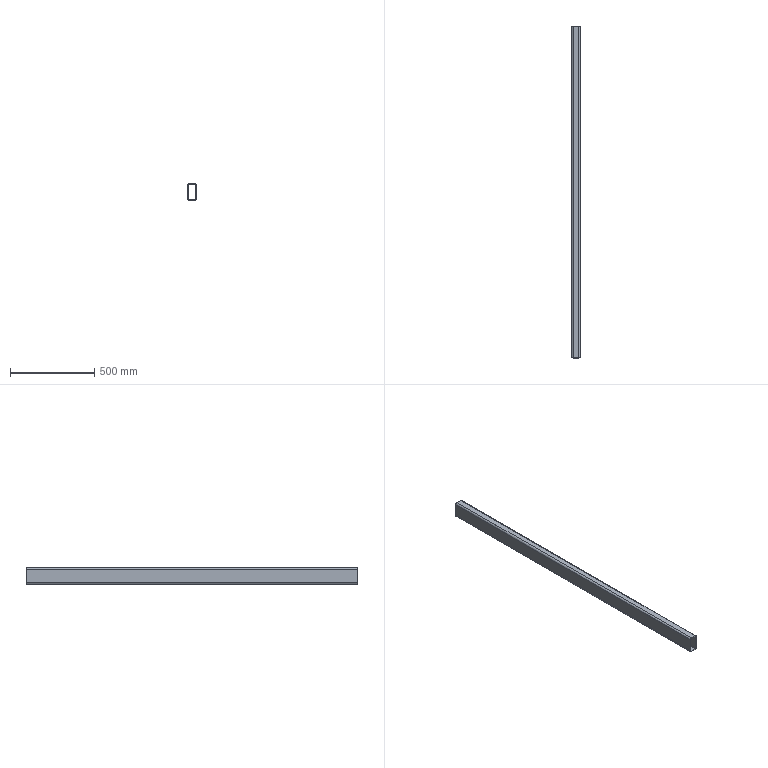Part | STEP file | E3-楼梯立柱主体-95_Default<As Machined> | 1 solid | 18 faces | box 50 x 1968 x 100 mm | volume 2127530 mm3 | plane 10 | cylinder 8 | commonest cylinder face diameters 12 x4 20 x4
STEP:
#1=CARTESIAN_POINT('',(0.,0.,0.));
#2=DIRECTION('',(0.,0.,1.));
#3=DIRECTION('',(1.,0.,0.));
#4=AXIS2_PLACEMENT_3D('',#1,#2,#3);
#5=CARTESIAN_POINT('',(-25.,0.,-40.));
#6=VERTEX_POINT('',#5);
#7=CARTESIAN_POINT('',(-15.,0.,-50.));
#8=VERTEX_POINT('',#7);
#9=CARTESIAN_POINT('',(-15.,0.,-40.));
#10=DIRECTION('',(0.,-1.,0.));
#11=DIRECTION('',(0.,0.,-1.));
#12=AXIS2_PLACEMENT_3D('',#9,#10,#11);
#13=CIRCLE('',#12,10.);
#14=CARTESIAN_POINT('',(-15.,1968.,-40.));
#15=DIRECTION('',(0.,-1.,0.));
#16=DIRECTION('',(0.,0.,1.));
#17=AXIS2_PLACEMENT_3D('',#14,#15,#16);
#18=CYLINDRICAL_SURFACE('',#17,10.);
#19=CARTESIAN_POINT('',(-3.142,1968.));
#20=DIRECTION('',(1.,0.));
#21=VECTOR('',#20,1.);
#22=LINE('',#19,#21);
#23=(GEOMETRIC_REPRESENTATION_CONTEXT(2)PARAMETRIC_REPRESENTATION_CONTEXT()REPRESENTATION_CONTEXT('',''));
#24=DEFINITIONAL_REPRESENTATION('',(#22),#23);
#25=PCURVE('',#18,#24);
#26=CARTESIAN_POINT('',(-15.,0.,-40.));
#27=DIRECTION('',(0.,1.,0.));
#28=DIRECTION('',(0.,0.,-1.));
#29=AXIS2_PLACEMENT_3D('',#26,#27,#28);
#30=PLANE('',#29);
#31=CARTESIAN_POINT('',(10.,0.));
#32=CARTESIAN_POINT('',(10.,-17.321));
#33=CARTESIAN_POINT('',(-5.,-8.66));
#34=CARTESIAN_POINT('',(-20.,0.));
#35=CARTESIAN_POINT('',(-5.,8.66));
#36=CARTESIAN_POINT('',(10.,17.321));
#37=CARTESIAN_POINT('',(10.,0.));
#38=(BOUNDED_CURVE()B_SPLINE_CURVE(2,(#31,#32,#33,#34,#35,#36,#37),.UNSPECIFIED.,.T.,.F.)B_SPLINE_CURVE_WITH_KNOTS((1,2,2,2,2,1),(-2.094,0.,2.094,4.189,6.283,8.378),.UNSPECIFIED.)CURVE()GEOMETRIC_REPRESENTATION_ITEM()RATIONAL_B_SPLINE_CURVE((1.,0.5,1.,0.5,1.,0.5,1.))REPRESENTATION_ITEM(''));
#39=(GEOMETRIC_REPRESENTATION_CONTEXT(2)PARAMETRIC_REPRESENTATION_CONTEXT()REPRESENTATION_CONTEXT('',''));
#40=DEFINITIONAL_REPRESENTATION('',(#38),#39);
#41=PCURVE('',#30,#40);
#42=SURFACE_CURVE('',#13,(#25,#41),.PCURVE_S1.);
#43=EDGE_CURVE('',#6,#8,#42,.T.);
#44=ORIENTED_EDGE('',*,*,#43,.F.);
#45=CARTESIAN_POINT('',(-25.,1968.,-40.));
#46=VERTEX_POINT('',#45);
#47=CARTESIAN_POINT('',(-25.,1968.,-40.));
#48=DIRECTION('',(0.,-1.,0.));
#49=VECTOR('',#48,1.);
#50=LINE('',#47,#49);
#51=CARTESIAN_POINT('',(1.571,0.));
#52=DIRECTION('',(0.,1.));
#53=VECTOR('',#52,1.);
#54=LINE('',#51,#53);
#55=(GEOMETRIC_REPRESENTATION_CONTEXT(2)PARAMETRIC_REPRESENTATION_CONTEXT()REPRESENTATION_CONTEXT('',''));
#56=DEFINITIONAL_REPRESENTATION('',(#54),#55);
#57=PCURVE('',#18,#56);
#58=CARTESIAN_POINT('',(-25.,1968.,-40.));
#59=DIRECTION('',(1.,0.,0.));
#60=DIRECTION('',(0.,0.,1.));
#61=AXIS2_PLACEMENT_3D('',#58,#59,#60);
#62=PLANE('',#61);
#63=CARTESIAN_POINT('',(0.,0.));
#64=DIRECTION('',(0.,1.));
#65=VECTOR('',#64,1.);
#66=LINE('',#63,#65);
#67=(GEOMETRIC_REPRESENTATION_CONTEXT(2)PARAMETRIC_REPRESENTATION_CONTEXT()REPRESENTATION_CONTEXT('',''));
#68=DEFINITIONAL_REPRESENTATION('',(#66),#67);
#69=PCURVE('',#62,#68);
#70=SURFACE_CURVE('',#50,(#57,#69),.PCURVE_S1.);
#71=EDGE_CURVE('',#46,#6,#70,.T.);
#72=ORIENTED_EDGE('',*,*,#71,.F.);
#73=CARTESIAN_POINT('',(-15.,1968.,-50.));
#74=VERTEX_POINT('',#73);
#75=CARTESIAN_POINT('',(-15.,1968.,-40.));
#76=DIRECTION('',(0.,-1.,0.));
#77=DIRECTION('',(0.,0.,-1.));
#78=AXIS2_PLACEMENT_3D('',#75,#76,#77);
#79=CIRCLE('',#78,10.);
#80=CARTESIAN_POINT('',(-3.142,0.));
#81=DIRECTION('',(1.,0.));
#82=VECTOR('',#81,1.);
#83=LINE('',#80,#82);
#84=(GEOMETRIC_REPRESENTATION_CONTEXT(2)PARAMETRIC_REPRESENTATION_CONTEXT()REPRESENTATION_CONTEXT('',''));
#85=DEFINITIONAL_REPRESENTATION('',(#83),#84);
#86=PCURVE('',#18,#85);
#87=CARTESIAN_POINT('',(-15.,1968.,-40.));
#88=DIRECTION('',(0.,1.,0.));
#89=DIRECTION('',(0.,0.,-1.));
#90=AXIS2_PLACEMENT_3D('',#87,#88,#89);
#91=PLANE('',#90);
#92=CARTESIAN_POINT('',(10.,0.));
#93=CARTESIAN_POINT('',(10.,-17.321));
#94=CARTESIAN_POINT('',(-5.,-8.66));
#95=CARTESIAN_POINT('',(-20.,0.));
#96=CARTESIAN_POINT('',(-5.,8.66));
#97=CARTESIAN_POINT('',(10.,17.321));
#98=CARTESIAN_POINT('',(10.,0.));
#99=(BOUNDED_CURVE()B_SPLINE_CURVE(2,(#92,#93,#94,#95,#96,#97,#98),.UNSPECIFIED.,.T.,.F.)B_SPLINE_CURVE_WITH_KNOTS((1,2,2,2,2,1),(-2.094,0.,2.094,4.189,6.283,8.378),.UNSPECIFIED.)CURVE()GEOMETRIC_REPRESENTATION_ITEM()RATIONAL_B_SPLINE_CURVE((1.,0.5,1.,0.5,1.,0.5,1.))REPRESENTATION_ITEM(''));
#100=(GEOMETRIC_REPRESENTATION_CONTEXT(2)PARAMETRIC_REPRESENTATION_CONTEXT()REPRESENTATION_CONTEXT('',''));
#101=DEFINITIONAL_REPRESENTATION('',(#99),#100);
#102=PCURVE('',#91,#101);
#103=SURFACE_CURVE('',#79,(#86,#102),.PCURVE_S1.);
#104=EDGE_CURVE('',#46,#74,#103,.T.);
#105=ORIENTED_EDGE('',*,*,#104,.T.);
#106=CARTESIAN_POINT('',(-15.,1968.,-50.));
#107=DIRECTION('',(0.,-1.,0.));
#108=VECTOR('',#107,1.);
#109=LINE('',#106,#108);
#110=CARTESIAN_POINT('',(3.142,0.));
#111=DIRECTION('',(0.,1.));
#112=VECTOR('',#111,1.);
#113=LINE('',#110,#112);
#114=(GEOMETRIC_REPRESENTATION_CONTEXT(2)PARAMETRIC_REPRESENTATION_CONTEXT()REPRESENTATION_CONTEXT('',''));
#115=DEFINITIONAL_REPRESENTATION('',(#113),#114);
#116=PCURVE('',#18,#115);
#117=CARTESIAN_POINT('',(-15.,1968.,-50.));
#118=DIRECTION('',(0.,0.,1.));
#119=DIRECTION('',(-1.,0.,0.));
#120=AXIS2_PLACEMENT_3D('',#117,#118,#119);
#121=PLANE('',#120);
#122=CARTESIAN_POINT('',(0.,0.));
#123=DIRECTION('',(0.,1.));
#124=VECTOR('',#123,1.);
#125=LINE('',#122,#124);
#126=(GEOMETRIC_REPRESENTATION_CONTEXT(2)PARAMETRIC_REPRESENTATION_CONTEXT()REPRESENTATION_CONTEXT('',''));
#127=DEFINITIONAL_REPRESENTATION('',(#125),#126);
#128=PCURVE('',#121,#127);
#129=SURFACE_CURVE('',#109,(#116,#128),.PCURVE_S1.);
#130=EDGE_CURVE('',#74,#8,#129,.T.);
#131=ORIENTED_EDGE('',*,*,#130,.T.);
#132=EDGE_LOOP('',(#44,#72,#105,#131));
#133=FACE_BOUND('',#132,.T.);
#134=ADVANCED_FACE('',(#133),#18,.T.);
#135=CARTESIAN_POINT('',(15.,0.,-50.));
#136=VERTEX_POINT('',#135);
#137=CARTESIAN_POINT('',(-15.,0.,-50.));
#138=DIRECTION('',(1.,0.,0.));
#139=VECTOR('',#138,1.);
#140=LINE('',#137,#139);
#141=CARTESIAN_POINT('',(0.,1968.));
#142=DIRECTION('',(-1.,0.));
#143=VECTOR('',#142,1.);
#144=LINE('',#141,#143);
#145=(GEOMETRIC_REPRESENTATION_CONTEXT(2)PARAMETRIC_REPRESENTATION_CONTEXT()REPRESENTATION_CONTEXT('',''));
#146=DEFINITIONAL_REPRESENTATION('',(#144),#145);
#147=PCURVE('',#121,#146);
#148=CARTESIAN_POINT('',(10.,0.));
#149=DIRECTION('',(0.,-1.));
#150=VECTOR('',#149,1.);
#151=LINE('',#148,#150);
#152=(GEOMETRIC_REPRESENTATION_CONTEXT(2)PARAMETRIC_REPRESENTATION_CONTEXT()REPRESENTATION_CONTEXT('',''));
#153=DEFINITIONAL_REPRESENTATION('',(#151),#152);
#154=PCURVE('',#30,#153);
#155=SURFACE_CURVE('',#140,(#147,#154),.PCURVE_S1.);
#156=EDGE_CURVE('',#8,#136,#155,.T.);
#157=ORIENTED_EDGE('',*,*,#156,.F.);
#158=ORIENTED_EDGE('',*,*,#130,.F.);
#159=CARTESIAN_POINT('',(15.,1968.,-50.));
#160=VERTEX_POINT('',#159);
#161=CARTESIAN_POINT('',(-15.,1968.,-50.));
#162=DIRECTION('',(1.,0.,0.));
#163=VECTOR('',#162,1.);
#164=LINE('',#161,#163);
#165=CARTESIAN_POINT('',(0.,0.));
#166=DIRECTION('',(-1.,0.));
#167=VECTOR('',#166,1.);
#168=LINE('',#165,#167);
#169=(GEOMETRIC_REPRESENTATION_CONTEXT(2)PARAMETRIC_REPRESENTATION_CONTEXT()REPRESENTATION_CONTEXT('',''));
#170=DEFINITIONAL_REPRESENTATION('',(#168),#169);
#171=PCURVE('',#121,#170);
#172=CARTESIAN_POINT('',(10.,0.));
#173=DIRECTION('',(0.,-1.));
#174=VECTOR('',#173,1.);
#175=LINE('',#172,#174);
#176=(GEOMETRIC_REPRESENTATION_CONTEXT(2)PARAMETRIC_REPRESENTATION_CONTEXT()REPRESENTATION_CONTEXT('',''));
#177=DEFINITIONAL_REPRESENTATION('',(#175),#176);
#178=PCURVE('',#91,#177);
#179=SURFACE_CURVE('',#164,(#171,#178),.PCURVE_S1.);
#180=EDGE_CURVE('',#74,#160,#179,.T.);
#181=ORIENTED_EDGE('',*,*,#180,.T.);
#182=CARTESIAN_POINT('',(15.,1968.,-50.));
#183=DIRECTION('',(0.,-1.,0.));
#184=VECTOR('',#183,1.);
#185=LINE('',#182,#184);
#186=CARTESIAN_POINT('',(-30.,0.));
#187=DIRECTION('',(0.,1.));
#188=VECTOR('',#187,1.);
#189=LINE('',#186,#188);
#190=(GEOMETRIC_REPRESENTATION_CONTEXT(2)PARAMETRIC_REPRESENTATION_CONTEXT()REPRESENTATION_CONTEXT('',''));
#191=DEFINITIONAL_REPRESENTATION('',(#189),#190);
#192=PCURVE('',#121,#191);
#193=CARTESIAN_POINT('',(15.,1968.,-40.));
#194=DIRECTION('',(0.,-1.,0.));
#195=DIRECTION('',(0.,0.,1.));
#196=AXIS2_PLACEMENT_3D('',#193,#194,#195);
#197=CYLINDRICAL_SURFACE('',#196,10.);
#198=CARTESIAN_POINT('',(3.142,0.));
#199=DIRECTION('',(0.,1.));
#200=VECTOR('',#199,1.);
#201=LINE('',#198,#200);
#202=(GEOMETRIC_REPRESENTATION_CONTEXT(2)PARAMETRIC_REPRESENTATION_CONTEXT()REPRESENTATION_CONTEXT('',''));
#203=DEFINITIONAL_REPRESENTATION('',(#201),#202);
#204=PCURVE('',#197,#203);
#205=SURFACE_CURVE('',#185,(#192,#204),.PCURVE_S1.);
#206=EDGE_CURVE('',#160,#136,#205,.T.);
#207=ORIENTED_EDGE('',*,*,#206,.T.);
#208=EDGE_LOOP('',(#157,#158,#181,#207));
#209=FACE_BOUND('',#208,.T.);
#210=ADVANCED_FACE('',(#209),#121,.F.);
#211=CARTESIAN_POINT('',(25.,0.,-40.));
#212=VERTEX_POINT('',#211);
#213=CARTESIAN_POINT('',(15.,0.,-40.));
#214=DIRECTION('',(0.,-1.,0.));
#215=DIRECTION('',(0.,0.,-1.));
#216=AXIS2_PLACEMENT_3D('',#213,#214,#215);
#217=CIRCLE('',#216,10.);
#218=CARTESIAN_POINT('',(3.142,1968.));
#219=DIRECTION('',(1.,0.));
#220=VECTOR('',#219,1.);
#221=LINE('',#218,#220);
#222=(GEOMETRIC_REPRESENTATION_CONTEXT(2)PARAMETRIC_REPRESENTATION_CONTEXT()REPRESENTATION_CONTEXT('',''));
#223=DEFINITIONAL_REPRESENTATION('',(#221),#222);
#224=PCURVE('',#197,#223);
#225=CARTESIAN_POINT('',(10.,-30.));
#226=CARTESIAN_POINT('',(10.,-47.321));
#227=CARTESIAN_POINT('',(-5.,-38.66));
#228=CARTESIAN_POINT('',(-20.,-30.));
#229=CARTESIAN_POINT('',(-5.,-21.34));
#230=CARTESIAN_POINT('',(10.,-12.679));
#231=CARTESIAN_POINT('',(10.,-30.));
#232=(BOUNDED_CURVE()B_SPLINE_CURVE(2,(#225,#226,#227,#228,#229,#230,#231),.UNSPECIFIED.,.T.,.F.)B_SPLINE_CURVE_WITH_KNOTS((1,2,2,2,2,1),(-2.094,0.,2.094,4.189,6.283,8.378),.UNSPECIFIED.)CURVE()GEOMETRIC_REPRESENTATION_ITEM()RATIONAL_B_SPLINE_CURVE((1.,0.5,1.,0.5,1.,0.5,1.))REPRESENTATION_ITEM(''));
#233=(GEOMETRIC_REPRESENTATION_CONTEXT(2)PARAMETRIC_REPRESENTATION_CONTEXT()REPRESENTATION_CONTEXT('',''));
#234=DEFINITIONAL_REPRESENTATION('',(#232),#233);
#235=PCURVE('',#30,#234);
#236=SURFACE_CURVE('',#217,(#224,#235),.PCURVE_S1.);
#237=EDGE_CURVE('',#136,#212,#236,.T.);
#238=ORIENTED_EDGE('',*,*,#237,.F.);
#239=ORIENTED_EDGE('',*,*,#206,.F.);
#240=CARTESIAN_POINT('',(25.,1968.,-40.));
#241=VERTEX_POINT('',#240);
#242=CARTESIAN_POINT('',(15.,1968.,-40.));
#243=DIRECTION('',(0.,-1.,0.));
#244=DIRECTION('',(0.,0.,-1.));
#245=AXIS2_PLACEMENT_3D('',#242,#243,#244);
#246=CIRCLE('',#245,10.);
#247=CARTESIAN_POINT('',(3.142,0.));
#248=DIRECTION('',(1.,0.));
#249=VECTOR('',#248,1.);
#250=LINE('',#247,#249);
#251=(GEOMETRIC_REPRESENTATION_CONTEXT(2)PARAMETRIC_REPRESENTATION_CONTEXT()REPRESENTATION_CONTEXT('',''));
#252=DEFINITIONAL_REPRESENTATION('',(#250),#251);
#253=PCURVE('',#197,#252);
#254=CARTESIAN_POINT('',(10.,-30.));
#255=CARTESIAN_POINT('',(10.,-47.321));
#256=CARTESIAN_POINT('',(-5.,-38.66));
#257=CARTESIAN_POINT('',(-20.,-30.));
#258=CARTESIAN_POINT('',(-5.,-21.34));
#259=CARTESIAN_POINT('',(10.,-12.679));
#260=CARTESIAN_POINT('',(10.,-30.));
#261=(BOUNDED_CURVE()B_SPLINE_CURVE(2,(#254,#255,#256,#257,#258,#259,#260),.UNSPECIFIED.,.T.,.F.)B_SPLINE_CURVE_WITH_KNOTS((1,2,2,2,2,1),(-2.094,0.,2.094,4.189,6.283,8.378),.UNSPECIFIED.)CURVE()GEOMETRIC_REPRESENTATION_ITEM()RATIONAL_B_SPLINE_CURVE((1.,0.5,1.,0.5,1.,0.5,1.))REPRESENTATION_ITEM(''));
#262=(GEOMETRIC_REPRESENTATION_CONTEXT(2)PARAMETRIC_REPRESENTATION_CONTEXT()REPRESENTATION_CONTEXT('',''));
#263=DEFINITIONAL_REPRESENTATION('',(#261),#262);
#264=PCURVE('',#91,#263);
#265=SURFACE_CURVE('',#246,(#253,#264),.PCURVE_S1.);
#266=EDGE_CURVE('',#160,#241,#265,.T.);
#267=ORIENTED_EDGE('',*,*,#266,.T.);
#268=CARTESIAN_POINT('',(25.,1968.,-40.));
#269=DIRECTION('',(0.,-1.,0.));
#270=VECTOR('',#269,1.);
#271=LINE('',#268,#270);
#272=CARTESIAN_POINT('',(4.712,0.));
#273=DIRECTION('',(0.,1.));
#274=VECTOR('',#273,1.);
#275=LINE('',#272,#274);
#276=(GEOMETRIC_REPRESENTATION_CONTEXT(2)PARAMETRIC_REPRESENTATION_CONTEXT()REPRESENTATION_CONTEXT('',''));
#277=DEFINITIONAL_REPRESENTATION('',(#275),#276);
#278=PCURVE('',#197,#277);
#279=CARTESIAN_POINT('',(25.,1968.,40.));
#280=DIRECTION('',(-1.,0.,0.));
#281=DIRECTION('',(0.,0.,-1.));
#282=AXIS2_PLACEMENT_3D('',#279,#280,#281);
#283=PLANE('',#282);
#284=CARTESIAN_POINT('',(80.,0.));
#285=DIRECTION('',(0.,1.));
#286=VECTOR('',#285,1.);
#287=LINE('',#284,#286);
#288=(GEOMETRIC_REPRESENTATION_CONTEXT(2)PARAMETRIC_REPRESENTATION_CONTEXT()REPRESENTATION_CONTEXT('',''));
#289=DEFINITIONAL_REPRESENTATION('',(#287),#288);
#290=PCURVE('',#283,#289);
#291=SURFACE_CURVE('',#271,(#278,#290),.PCURVE_S1.);
#292=EDGE_CURVE('',#241,#212,#291,.T.);
#293=ORIENTED_EDGE('',*,*,#292,.T.);
#294=EDGE_LOOP('',(#238,#239,#267,#293));
#295=FACE_BOUND('',#294,.T.);
#296=ADVANCED_FACE('',(#295),#197,.T.);
#297=CARTESIAN_POINT('',(25.,0.,40.));
#298=VERTEX_POINT('',#297);
#299=CARTESIAN_POINT('',(25.,0.,40.));
#300=DIRECTION('',(0.,0.,1.));
#301=VECTOR('',#300,1.);
#302=LINE('',#299,#301);
#303=CARTESIAN_POINT('',(0.,1968.));
#304=DIRECTION('',(-1.,0.));
#305=VECTOR('',#304,1.);
#306=LINE('',#303,#305);
#307=(GEOMETRIC_REPRESENTATION_CONTEXT(2)PARAMETRIC_REPRESENTATION_CONTEXT()REPRESENTATION_CONTEXT('',''));
#308=DEFINITIONAL_REPRESENTATION('',(#306),#307);
#309=PCURVE('',#283,#308);
#310=CARTESIAN_POINT('',(-80.,-40.));
#311=DIRECTION('',(-1.,0.));
#312=VECTOR('',#311,1.);
#313=LINE('',#310,#312);
#314=(GEOMETRIC_REPRESENTATION_CONTEXT(2)PARAMETRIC_REPRESENTATION_CONTEXT()REPRESENTATION_CONTEXT('',''));
#315=DEFINITIONAL_REPRESENTATION('',(#313),#314);
#316=PCURVE('',#30,#315);
#317=SURFACE_CURVE('',#302,(#309,#316),.PCURVE_S1.);
#318=EDGE_CURVE('',#212,#298,#317,.T.);
#319=ORIENTED_EDGE('',*,*,#318,.F.);
#320=ORIENTED_EDGE('',*,*,#292,.F.);
#321=CARTESIAN_POINT('',(25.,1968.,40.));
#322=VERTEX_POINT('',#321);
#323=CARTESIAN_POINT('',(25.,1968.,40.));
#324=DIRECTION('',(0.,0.,1.));
#325=VECTOR('',#324,1.);
#326=LINE('',#323,#325);
#327=CARTESIAN_POINT('',(0.,0.));
#328=DIRECTION('',(-1.,0.));
#329=VECTOR('',#328,1.);
#330=LINE('',#327,#329);
#331=(GEOMETRIC_REPRESENTATION_CONTEXT(2)PARAMETRIC_REPRESENTATION_CONTEXT()REPRESENTATION_CONTEXT('',''));
#332=DEFINITIONAL_REPRESENTATION('',(#330),#331);
#333=PCURVE('',#283,#332);
#334=CARTESIAN_POINT('',(-80.,-40.));
#335=DIRECTION('',(-1.,0.));
#336=VECTOR('',#335,1.);
#337=LINE('',#334,#336);
#338=(GEOMETRIC_REPRESENTATION_CONTEXT(2)PARAMETRIC_REPRESENTATION_CONTEXT()REPRESENTATION_CONTEXT('',''));
#339=DEFINITIONAL_REPRESENTATION('',(#337),#338);
#340=PCURVE('',#91,#339);
#341=SURFACE_CURVE('',#326,(#333,#340),.PCURVE_S1.);
#342=EDGE_CURVE('',#241,#322,#341,.T.);
#343=ORIENTED_EDGE('',*,*,#342,.T.);
#344=CARTESIAN_POINT('',(25.,1968.,40.));
#345=DIRECTION('',(0.,-1.,0.));
#346=VECTOR('',#345,1.);
#347=LINE('',#344,#346);
#348=CARTESIAN_POINT('',(0.,0.));
#349=DIRECTION('',(0.,1.));
#350=VECTOR('',#349,1.);
#351=LINE('',#348,#350);
#352=(GEOMETRIC_REPRESENTATION_CONTEXT(2)PARAMETRIC_REPRESENTATION_CONTEXT()REPRESENTATION_CONTEXT('',''));
#353=DEFINITIONAL_REPRESENTATION('',(#351),#352);
#354=PCURVE('',#283,#353);
#355=CARTESIAN_POINT('',(15.,1968.,40.));
#356=DIRECTION('',(0.,-1.,0.));
#357=DIRECTION('',(0.,0.,1.));
#358=AXIS2_PLACEMENT_3D('',#355,#356,#357);
#359=CYLINDRICAL_SURFACE('',#358,10.);
#360=CARTESIAN_POINT('',(4.712,0.));
#361=DIRECTION('',(0.,1.));
#362=VECTOR('',#361,1.);
#363=LINE('',#360,#362);
#364=(GEOMETRIC_REPRESENTATION_CONTEXT(2)PARAMETRIC_REPRESENTATION_CONTEXT()REPRESENTATION_CONTEXT('',''));
#365=DEFINITIONAL_REPRESENTATION('',(#363),#364);
#366=PCURVE('',#359,#365);
#367=SURFACE_CURVE('',#347,(#354,#366),.PCURVE_S1.);
#368=EDGE_CURVE('',#322,#298,#367,.T.);
#369=ORIENTED_EDGE('',*,*,#368,.T.);
#370=EDGE_LOOP('',(#319,#320,#343,#369));
#371=FACE_BOUND('',#370,.T.);
#372=ADVANCED_FACE('',(#371),#283,.F.);
#373=CARTESIAN_POINT('',(15.,0.,50.));
#374=VERTEX_POINT('',#373);
#375=CARTESIAN_POINT('',(15.,0.,40.));
#376=DIRECTION('',(0.,-1.,0.));
#377=DIRECTION('',(0.,0.,-1.));
#378=AXIS2_PLACEMENT_3D('',#375,#376,#377);
#379=CIRCLE('',#378,10.);
#380=CARTESIAN_POINT('',(3.142,1968.));
#381=DIRECTION('',(1.,0.));
#382=VECTOR('',#381,1.);
#383=LINE('',#380,#382);
#384=(GEOMETRIC_REPRESENTATION_CONTEXT(2)PARAMETRIC_REPRESENTATION_CONTEXT()REPRESENTATION_CONTEXT('',''));
#385=DEFINITIONAL_REPRESENTATION('',(#383),#384);
#386=PCURVE('',#359,#385);
#387=CARTESIAN_POINT('',(-70.,-30.));
#388=CARTESIAN_POINT('',(-70.,-47.321));
#389=CARTESIAN_POINT('',(-85.,-38.66));
#390=CARTESIAN_POINT('',(-100.,-30.));
#391=CARTESIAN_POINT('',(-85.,-21.34));
#392=CARTESIAN_POINT('',(-70.,-12.679));
#393=CARTESIAN_POINT('',(-70.,-30.));
#394=(BOUNDED_CURVE()B_SPLINE_CURVE(2,(#387,#388,#389,#390,#391,#392,#393),.UNSPECIFIED.,.T.,.F.)B_SPLINE_CURVE_WITH_KNOTS((1,2,2,2,2,1),(-2.094,0.,2.094,4.189,6.283,8.378),.UNSPECIFIED.)CURVE()GEOMETRIC_REPRESENTATION_ITEM()RATIONAL_B_SPLINE_CURVE((1.,0.5,1.,0.5,1.,0.5,1.))REPRESENTATION_ITEM(''));
#395=(GEOMETRIC_REPRESENTATION_CONTEXT(2)PARAMETRIC_REPRESENTATION_CONTEXT()REPRESENTATION_CONTEXT('',''));
#396=DEFINITIONAL_REPRESENTATION('',(#394),#395);
#397=PCURVE('',#30,#396);
#398=SURFACE_CURVE('',#379,(#386,#397),.PCURVE_S1.);
#399=EDGE_CURVE('',#298,#374,#398,.T.);
#400=ORIENTED_EDGE('',*,*,#399,.F.);
#401=ORIENTED_EDGE('',*,*,#368,.F.);
#402=CARTESIAN_POINT('',(15.,1968.,50.));
#403=VERTEX_POINT('',#402);
#404=CARTESIAN_POINT('',(15.,1968.,40.));
#405=DIRECTION('',(0.,-1.,0.));
#406=DIRECTION('',(0.,0.,-1.));
#407=AXIS2_PLACEMENT_3D('',#404,#405,#406);
#408=CIRCLE('',#407,10.);
#409=CARTESIAN_POINT('',(3.142,0.));
#410=DIRECTION('',(1.,0.));
#411=VECTOR('',#410,1.);
#412=LINE('',#409,#411);
#413=(GEOMETRIC_REPRESENTATION_CONTEXT(2)PARAMETRIC_REPRESENTATION_CONTEXT()REPRESENTATION_CONTEXT('',''));
#414=DEFINITIONAL_REPRESENTATION('',(#412),#413);
#415=PCURVE('',#359,#414);
#416=CARTESIAN_POINT('',(-70.,-30.));
#417=CARTESIAN_POINT('',(-70.,-47.321));
#418=CARTESIAN_POINT('',(-85.,-38.66));
#419=CARTESIAN_POINT('',(-100.,-30.));
#420=CARTESIAN_POINT('',(-85.,-21.34));
#421=CARTESIAN_POINT('',(-70.,-12.679));
#422=CARTESIAN_POINT('',(-70.,-30.));
#423=(BOUNDED_CURVE()B_SPLINE_CURVE(2,(#416,#417,#418,#419,#420,#421,#422),.UNSPECIFIED.,.T.,.F.)B_SPLINE_CURVE_WITH_KNOTS((1,2,2,2,2,1),(-2.094,0.,2.094,4.189,6.283,8.378),.UNSPECIFIED.)CURVE()GEOMETRIC_REPRESENTATION_ITEM()RATIONAL_B_SPLINE_CURVE((1.,0.5,1.,0.5,1.,0.5,1.))REPRESENTATION_ITEM(''));
#424=(GEOMETRIC_REPRESENTATION_CONTEXT(2)PARAMETRIC_REPRESENTATION_CONTEXT()REPRESENTATION_CONTEXT('',''));
#425=DEFINITIONAL_REPRESENTATION('',(#423),#424);
#426=PCURVE('',#91,#425);
#427=SURFACE_CURVE('',#408,(#415,#426),.PCURVE_S1.);
#428=EDGE_CURVE('',#322,#403,#427,.T.);
#429=ORIENTED_EDGE('',*,*,#428,.T.);
#430=CARTESIAN_POINT('',(15.,1968.,50.));
#431=DIRECTION('',(0.,-1.,0.));
#432=VECTOR('',#431,1.);
#433=LINE('',#430,#432);
#434=CARTESIAN_POINT('',(6.283,0.));
#435=DIRECTION('',(0.,1.));
#436=VECTOR('',#435,1.);
#437=LINE('',#434,#436);
#438=(GEOMETRIC_REPRESENTATION_CONTEXT(2)PARAMETRIC_REPRESENTATION_CONTEXT()REPRESENTATION_CONTEXT('',''));
#439=DEFINITIONAL_REPRESENTATION('',(#437),#438);
#440=PCURVE('',#359,#439);
#441=CARTESIAN_POINT('',(15.,1968.,50.));
#442=DIRECTION('',(0.,0.,-1.));
#443=DIRECTION('',(1.,0.,0.));
#444=AXIS2_PLACEMENT_3D('',#441,#442,#443);
#445=PLANE('',#444);
#446=CARTESIAN_POINT('',(0.,0.));
#447=DIRECTION('',(0.,1.));
#448=VECTOR('',#447,1.);
#449=LINE('',#446,#448);
#450=(GEOMETRIC_REPRESENTATION_CONTEXT(2)PARAMETRIC_REPRESENTATION_CONTEXT()REPRESENTATION_CONTEXT('',''));
#451=DEFINITIONAL_REPRESENTATION('',(#449),#450);
#452=PCURVE('',#445,#451);
#453=SURFACE_CURVE('',#433,(#440,#452),.PCURVE_S1.);
#454=EDGE_CURVE('',#403,#374,#453,.T.);
#455=ORIENTED_EDGE('',*,*,#454,.T.);
#456=EDGE_LOOP('',(#400,#401,#429,#455));
#457=FACE_BOUND('',#456,.T.);
#458=ADVANCED_FACE('',(#457),#359,.T.);
#459=CARTESIAN_POINT('',(-15.,0.,50.));
#460=VERTEX_POINT('',#459);
#461=CARTESIAN_POINT('',(15.,0.,50.));
#462=DIRECTION('',(-1.,0.,0.));
#463=VECTOR('',#462,1.);
#464=LINE('',#461,#463);
#465=CARTESIAN_POINT('',(0.,1968.));
#466=DIRECTION('',(-1.,0.));
#467=VECTOR('',#466,1.);
#468=LINE('',#465,#467);
#469=(GEOMETRIC_REPRESENTATION_CONTEXT(2)PARAMETRIC_REPRESENTATION_CONTEXT()REPRESENTATION_CONTEXT('',''));
#470=DEFINITIONAL_REPRESENTATION('',(#468),#469);
#471=PCURVE('',#445,#470);
#472=CARTESIAN_POINT('',(-90.,-30.));
#473=DIRECTION('',(0.,1.));
#474=VECTOR('',#473,1.);
#475=LINE('',#472,#474);
#476=(GEOMETRIC_REPRESENTATION_CONTEXT(2)PARAMETRIC_REPRESENTATION_CONTEXT()REPRESENTATION_CONTEXT('',''));
#477=DEFINITIONAL_REPRESENTATION('',(#475),#476);
#478=PCURVE('',#30,#477);
#479=SURFACE_CURVE('',#464,(#471,#478),.PCURVE_S1.);
#480=EDGE_CURVE('',#374,#460,#479,.T.);
#481=ORIENTED_EDGE('',*,*,#480,.F.);
#482=ORIENTED_EDGE('',*,*,#454,.F.);
#483=CARTESIAN_POINT('',(-15.,1968.,50.));
#484=VERTEX_POINT('',#483);
#485=CARTESIAN_POINT('',(15.,1968.,50.));
#486=DIRECTION('',(-1.,0.,0.));
#487=VECTOR('',#486,1.);
#488=LINE('',#485,#487);
#489=CARTESIAN_POINT('',(0.,0.));
#490=DIRECTION('',(-1.,0.));
#491=VECTOR('',#490,1.);
#492=LINE('',#489,#491);
#493=(GEOMETRIC_REPRESENTATION_CONTEXT(2)PARAMETRIC_REPRESENTATION_CONTEXT()REPRESENTATION_CONTEXT('',''));
#494=DEFINITIONAL_REPRESENTATION('',(#492),#493);
#495=PCURVE('',#445,#494);
#496=CARTESIAN_POINT('',(-90.,-30.));
#497=DIRECTION('',(0.,1.));
#498=VECTOR('',#497,1.);
#499=LINE('',#496,#498);
#500=(GEOMETRIC_REPRESENTATION_CONTEXT(2)PARAMETRIC_REPRESENTATION_CONTEXT()REPRESENTATION_CONTEXT('',''));
#501=DEFINITIONAL_REPRESENTATION('',(#499),#500);
#502=PCURVE('',#91,#501);
#503=SURFACE_CURVE('',#488,(#495,#502),.PCURVE_S1.);
#504=EDGE_CURVE('',#403,#484,#503,.T.);
#505=ORIENTED_EDGE('',*,*,#504,.T.);
#506=CARTESIAN_POINT('',(-15.,1968.,50.));
#507=DIRECTION('',(0.,-1.,0.));
#508=VECTOR('',#507,1.);
#509=LINE('',#506,#508);
#510=CARTESIAN_POINT('',(-30.,0.));
#511=DIRECTION('',(0.,1.));
#512=VECTOR('',#511,1.);
#513=LINE('',#510,#512);
#514=(GEOMETRIC_REPRESENTATION_CONTEXT(2)PARAMETRIC_REPRESENTATION_CONTEXT()REPRESENTATION_CONTEXT('',''));
#515=DEFINITIONAL_REPRESENTATION('',(#513),#514);
#516=PCURVE('',#445,#515);
#517=CARTESIAN_POINT('',(-15.,1968.,40.));
#518=DIRECTION('',(0.,-1.,0.));
#519=DIRECTION('',(0.,0.,1.));
#520=AXIS2_PLACEMENT_3D('',#517,#518,#519);
#521=CYLINDRICAL_SURFACE('',#520,10.);
#522=CARTESIAN_POINT('',(0.,0.));
#523=DIRECTION('',(0.,1.));
#524=VECTOR('',#523,1.);
#525=LINE('',#522,#524);
#526=(GEOMETRIC_REPRESENTATION_CONTEXT(2)PARAMETRIC_REPRESENTATION_CONTEXT()REPRESENTATION_CONTEXT('',''));
#527=DEFINITIONAL_REPRESENTATION('',(#525),#526);
#528=PCURVE('',#521,#527);
#529=SURFACE_CURVE('',#509,(#516,#528),.PCURVE_S1.);
#530=EDGE_CURVE('',#484,#460,#529,.T.);
#531=ORIENTED_EDGE('',*,*,#530,.T.);
#532=EDGE_LOOP('',(#481,#482,#505,#531));
#533=FACE_BOUND('',#532,.T.);
#534=ADVANCED_FACE('',(#533),#445,.F.);
#535=CARTESIAN_POINT('',(-25.,0.,40.));
#536=VERTEX_POINT('',#535);
#537=CARTESIAN_POINT('',(-15.,0.,40.));
#538=DIRECTION('',(0.,-1.,0.));
#539=DIRECTION('',(0.,0.,-1.));
#540=AXIS2_PLACEMENT_3D('',#537,#538,#539);
#541=CIRCLE('',#540,10.);
#542=CARTESIAN_POINT('',(-3.142,1968.));
#543=DIRECTION('',(1.,0.));
#544=VECTOR('',#543,1.);
#545=LINE('',#542,#544);
#546=(GEOMETRIC_REPRESENTATION_CONTEXT(2)PARAMETRIC_REPRESENTATION_CONTEXT()REPRESENTATION_CONTEXT('',''));
#547=DEFINITIONAL_REPRESENTATION('',(#545),#546);
#548=PCURVE('',#521,#547);
#549=CARTESIAN_POINT('',(-70.,0.));
#550=CARTESIAN_POINT('',(-70.,-17.321));
#551=CARTESIAN_POINT('',(-85.,-8.66));
#552=CARTESIAN_POINT('',(-100.,0.));
#553=CARTESIAN_POINT('',(-85.,8.66));
#554=CARTESIAN_POINT('',(-70.,17.321));
#555=CARTESIAN_POINT('',(-70.,0.));
#556=(BOUNDED_CURVE()B_SPLINE_CURVE(2,(#549,#550,#551,#552,#553,#554,#555),.UNSPECIFIED.,.T.,.F.)B_SPLINE_CURVE_WITH_KNOTS((1,2,2,2,2,1),(-2.094,0.,2.094,4.189,6.283,8.378),.UNSPECIFIED.)CURVE()GEOMETRIC_REPRESENTATION_ITEM()RATIONAL_B_SPLINE_CURVE((1.,0.5,1.,0.5,1.,0.5,1.))REPRESENTATION_ITEM(''));
#557=(GEOMETRIC_REPRESENTATION_CONTEXT(2)PARAMETRIC_REPRESENTATION_CONTEXT()REPRESENTATION_CONTEXT('',''));
#558=DEFINITIONAL_REPRESENTATION('',(#556),#557);
#559=PCURVE('',#30,#558);
#560=SURFACE_CURVE('',#541,(#548,#559),.PCURVE_S1.);
#561=EDGE_CURVE('',#460,#536,#560,.T.);
#562=ORIENTED_EDGE('',*,*,#561,.F.);
#563=ORIENTED_EDGE('',*,*,#530,.F.);
#564=CARTESIAN_POINT('',(-25.,1968.,40.));
#565=VERTEX_POINT('',#564);
#566=CARTESIAN_POINT('',(-15.,1968.,40.));
#567=DIRECTION('',(0.,-1.,0.));
#568=DIRECTION('',(0.,0.,-1.));
#569=AXIS2_PLACEMENT_3D('',#566,#567,#568);
#570=CIRCLE('',#569,10.);
#571=CARTESIAN_POINT('',(-3.142,0.));
#572=DIRECTION('',(1.,0.));
#573=VECTOR('',#572,1.);
#574=LINE('',#571,#573);
#575=(GEOMETRIC_REPRESENTATION_CONTEXT(2)PARAMETRIC_REPRESENTATION_CONTEXT()REPRESENTATION_CONTEXT('',''));
#576=DEFINITIONAL_REPRESENTATION('',(#574),#575);
#577=PCURVE('',#521,#576);
#578=CARTESIAN_POINT('',(-70.,0.));
#579=CARTESIAN_POINT('',(-70.,-17.321));
#580=CARTESIAN_POINT('',(-85.,-8.66));
#581=CARTESIAN_POINT('',(-100.,0.));
#582=CARTESIAN_POINT('',(-85.,8.66));
#583=CARTESIAN_POINT('',(-70.,17.321));
#584=CARTESIAN_POINT('',(-70.,0.));
#585=(BOUNDED_CURVE()B_SPLINE_CURVE(2,(#578,#579,#580,#581,#582,#583,#584),.UNSPECIFIED.,.T.,.F.)B_SPLINE_CURVE_WITH_KNOTS((1,2,2,2,2,1),(-2.094,0.,2.094,4.189,6.283,8.378),.UNSPECIFIED.)CURVE()GEOMETRIC_REPRESENTATION_ITEM()RATIONAL_B_SPLINE_CURVE((1.,0.5,1.,0.5,1.,0.5,1.))REPRESENTATION_ITEM(''));
#586=(GEOMETRIC_REPRESENTATION_CONTEXT(2)PARAMETRIC_REPRESENTATION_CONTEXT()REPRESENTATION_CONTEXT('',''));
#587=DEFINITIONAL_REPRESENTATION('',(#585),#586);
#588=PCURVE('',#91,#587);
#589=SURFACE_CURVE('',#570,(#577,#588),.PCURVE_S1.);
#590=EDGE_CURVE('',#484,#565,#589,.T.);
#591=ORIENTED_EDGE('',*,*,#590,.T.);
#592=CARTESIAN_POINT('',(-25.,1968.,40.));
#593=DIRECTION('',(0.,-1.,0.));
#594=VECTOR('',#593,1.);
#595=LINE('',#592,#594);
#596=CARTESIAN_POINT('',(1.571,0.));
#597=DIRECTION('',(0.,1.));
#598=VECTOR('',#597,1.);
#599=LINE('',#596,#598);
#600=(GEOMETRIC_REPRESENTATION_CONTEXT(2)PARAMETRIC_REPRESENTATION_CONTEXT()REPRESENTATION_CONTEXT('',''));
#601=DEFINITIONAL_REPRESENTATION('',(#599),#600);
#602=PCURVE('',#521,#601);
#603=CARTESIAN_POINT('',(80.,0.));
#604=DIRECTION('',(0.,1.));
#605=VECTOR('',#604,1.);
#606=LINE('',#603,#605);
#607=(GEOMETRIC_REPRESENTATION_CONTEXT(2)PARAMETRIC_REPRESENTATION_CONTEXT()REPRESENTATION_CONTEXT('',''));
#608=DEFINITIONAL_REPRESENTATION('',(#606),#607);
#609=PCURVE('',#62,#608);
#610=SURFACE_CURVE('',#595,(#602,#609),.PCURVE_S1.);
#611=EDGE_CURVE('',#565,#536,#610,.T.);
#612=ORIENTED_EDGE('',*,*,#611,.T.);
#613=EDGE_LOOP('',(#562,#563,#591,#612));
#614=FACE_BOUND('',#613,.T.);
#615=ADVANCED_FACE('',(#614),#521,.T.);
#616=CARTESIAN_POINT('',(15.,1968.,-46.));
#617=VERTEX_POINT('',#616);
#618=CARTESIAN_POINT('',(15.,0.,-46.));
#619=VERTEX_POINT('',#618);
#620=CARTESIAN_POINT('',(15.,1968.,-46.));
#621=DIRECTION('',(0.,-1.,0.));
#622=VECTOR('',#621,1.);
#623=LINE('',#620,#622);
#624=CARTESIAN_POINT('',(15.,1968.,-40.));
#625=DIRECTION('',(0.,-1.,0.));
#626=DIRECTION('',(0.,0.,1.));
#627=AXIS2_PLACEMENT_3D('',#624,#625,#626);
#628=CYLINDRICAL_SURFACE('',#627,6.);
#629=CARTESIAN_POINT('',(3.142,0.));
#630=DIRECTION('',(0.,1.));
#631=VECTOR('',#630,1.);
#632=LINE('',#629,#631);
#633=(GEOMETRIC_REPRESENTATION_CONTEXT(2)PARAMETRIC_REPRESENTATION_CONTEXT()REPRESENTATION_CONTEXT('',''));
#634=DEFINITIONAL_REPRESENTATION('',(#632),#633);
#635=PCURVE('',#628,#634);
#636=CARTESIAN_POINT('',(-15.,1968.,-46.));
#637=DIRECTION('',(0.,0.,1.));
#638=DIRECTION('',(-1.,0.,0.));
#639=AXIS2_PLACEMENT_3D('',#636,#637,#638);
#640=PLANE('',#639);
#641=CARTESIAN_POINT('',(-30.,0.));
#642=DIRECTION('',(0.,1.));
#643=VECTOR('',#642,1.);
#644=LINE('',#641,#643);
#645=(GEOMETRIC_REPRESENTATION_CONTEXT(2)PARAMETRIC_REPRESENTATION_CONTEXT()REPRESENTATION_CONTEXT('',''));
#646=DEFINITIONAL_REPRESENTATION('',(#644),#645);
#647=PCURVE('',#640,#646);
#648=SURFACE_CURVE('',#623,(#635,#647),.PCURVE_S1.);
#649=EDGE_CURVE('',#617,#619,#648,.T.);
#650=ORIENTED_EDGE('',*,*,#649,.F.);
#651=CARTESIAN_POINT('',(21.,1968.,-40.));
#652=VERTEX_POINT('',#651);
#653=CARTESIAN_POINT('',(15.,1968.,-40.));
#654=DIRECTION('',(0.,-1.,0.));
#655=DIRECTION('',(0.,0.,-1.));
#656=AXIS2_PLACEMENT_3D('',#653,#654,#655);
#657=CIRCLE('',#656,6.);
#658=CARTESIAN_POINT('',(3.142,0.));
#659=DIRECTION('',(1.,0.));
#660=VECTOR('',#659,1.);
#661=LINE('',#658,#660);
#662=(GEOMETRIC_REPRESENTATION_CONTEXT(2)PARAMETRIC_REPRESENTATION_CONTEXT()REPRESENTATION_CONTEXT('',''));
#663=DEFINITIONAL_REPRESENTATION('',(#661),#662);
#664=PCURVE('',#628,#663);
#665=CARTESIAN_POINT('',(6.,-30.));
#666=CARTESIAN_POINT('',(6.,-40.392));
#667=CARTESIAN_POINT('',(-3.,-35.196));
#668=CARTESIAN_POINT('',(-12.,-30.));
#669=CARTESIAN_POINT('',(-3.,-24.804));
#670=CARTESIAN_POINT('',(6.,-19.608));
#671=CARTESIAN_POINT('',(6.,-30.));
#672=(BOUNDED_CURVE()B_SPLINE_CURVE(2,(#665,#666,#667,#668,#669,#670,#671),.UNSPECIFIED.,.T.,.F.)B_SPLINE_CURVE_WITH_KNOTS((1,2,2,2,2,1),(-2.094,0.,2.094,4.189,6.283,8.378),.UNSPECIFIED.)CURVE()GEOMETRIC_REPRESENTATION_ITEM()RATIONAL_B_SPLINE_CURVE((1.,0.5,1.,0.5,1.,0.5,1.))REPRESENTATION_ITEM(''));
#673=(GEOMETRIC_REPRESENTATION_CONTEXT(2)PARAMETRIC_REPRESENTATION_CONTEXT()REPRESENTATION_CONTEXT('',''));
#674=DEFINITIONAL_REPRESENTATION('',(#672),#673);
#675=PCURVE('',#91,#674);
#676=SURFACE_CURVE('',#657,(#664,#675),.PCURVE_S1.);
#677=EDGE_CURVE('',#617,#652,#676,.T.);
#678=ORIENTED_EDGE('',*,*,#677,.T.);
#679=CARTESIAN_POINT('',(21.,0.,-40.));
#680=VERTEX_POINT('',#679);
#681=CARTESIAN_POINT('',(21.,1968.,-40.));
#682=DIRECTION('',(0.,-1.,0.));
#683=VECTOR('',#682,1.);
#684=LINE('',#681,#683);
#685=CARTESIAN_POINT('',(4.712,0.));
#686=DIRECTION('',(0.,1.));
#687=VECTOR('',#686,1.);
#688=LINE('',#685,#687);
#689=(GEOMETRIC_REPRESENTATION_CONTEXT(2)PARAMETRIC_REPRESENTATION_CONTEXT()REPRESENTATION_CONTEXT('',''));
#690=DEFINITIONAL_REPRESENTATION('',(#688),#689);
#691=PCURVE('',#628,#690);
#692=CARTESIAN_POINT('',(21.,1968.,40.));
#693=DIRECTION('',(-1.,0.,0.));
#694=DIRECTION('',(0.,0.,-1.));
#695=AXIS2_PLACEMENT_3D('',#692,#693,#694);
#696=PLANE('',#695);
#697=CARTESIAN_POINT('',(80.,0.));
#698=DIRECTION('',(0.,1.));
#699=VECTOR('',#698,1.);
#700=LINE('',#697,#699);
#701=(GEOMETRIC_REPRESENTATION_CONTEXT(2)PARAMETRIC_REPRESENTATION_CONTEXT()REPRESENTATION_CONTEXT('',''));
#702=DEFINITIONAL_REPRESENTATION('',(#700),#701);
#703=PCURVE('',#696,#702);
#704=SURFACE_CURVE('',#684,(#691,#703),.PCURVE_S1.);
#705=EDGE_CURVE('',#652,#680,#704,.T.);
#706=ORIENTED_EDGE('',*,*,#705,.T.);
#707=CARTESIAN_POINT('',(15.,0.,-40.));
#708=DIRECTION('',(0.,-1.,0.));
#709=DIRECTION('',(0.,0.,-1.));
#710=AXIS2_PLACEMENT_3D('',#707,#708,#709);
#711=CIRCLE('',#710,6.);
#712=CARTESIAN_POINT('',(3.142,1968.));
#713=DIRECTION('',(1.,0.));
#714=VECTOR('',#713,1.);
#715=LINE('',#712,#714);
#716=(GEOMETRIC_REPRESENTATION_CONTEXT(2)PARAMETRIC_REPRESENTATION_CONTEXT()REPRESENTATION_CONTEXT('',''));
#717=DEFINITIONAL_REPRESENTATION('',(#715),#716);
#718=PCURVE('',#628,#717);
#719=CARTESIAN_POINT('',(6.,-30.));
#720=CARTESIAN_POINT('',(6.,-40.392));
#721=CARTESIAN_POINT('',(-3.,-35.196));
#722=CARTESIAN_POINT('',(-12.,-30.));
#723=CARTESIAN_POINT('',(-3.,-24.804));
#724=CARTESIAN_POINT('',(6.,-19.608));
#725=CARTESIAN_POINT('',(6.,-30.));
#726=(BOUNDED_CURVE()B_SPLINE_CURVE(2,(#719,#720,#721,#722,#723,#724,#725),.UNSPECIFIED.,.T.,.F.)B_SPLINE_CURVE_WITH_KNOTS((1,2,2,2,2,1),(-2.094,0.,2.094,4.189,6.283,8.378),.UNSPECIFIED.)CURVE()GEOMETRIC_REPRESENTATION_ITEM()RATIONAL_B_SPLINE_CURVE((1.,0.5,1.,0.5,1.,0.5,1.))REPRESENTATION_ITEM(''));
#727=(GEOMETRIC_REPRESENTATION_CONTEXT(2)PARAMETRIC_REPRESENTATION_CONTEXT()REPRESENTATION_CONTEXT('',''));
#728=DEFINITIONAL_REPRESENTATION('',(#726),#727);
#729=PCURVE('',#30,#728);
#730=SURFACE_CURVE('',#711,(#718,#729),.PCURVE_S1.);
#731=EDGE_CURVE('',#619,#680,#730,.T.);
#732=ORIENTED_EDGE('',*,*,#731,.F.);
#733=EDGE_LOOP('',(#650,#678,#706,#732));
#734=FACE_BOUND('',#733,.F.);
#735=ADVANCED_FACE('',(#734),#628,.F.);
#736=CARTESIAN_POINT('',(-15.,0.,-46.));
#737=VERTEX_POINT('',#736);
#738=CARTESIAN_POINT('',(-15.,0.,-46.));
#739=DIRECTION('',(1.,0.,0.));
#740=VECTOR('',#739,1.);
#741=LINE('',#738,#740);
#742=CARTESIAN_POINT('',(0.,1968.));
#743=DIRECTION('',(-1.,0.));
#744=VECTOR('',#743,1.);
#745=LINE('',#742,#744);
#746=(GEOMETRIC_REPRESENTATION_CONTEXT(2)PARAMETRIC_REPRESENTATION_CONTEXT()REPRESENTATION_CONTEXT('',''));
#747=DEFINITIONAL_REPRESENTATION('',(#745),#746);
#748=PCURVE('',#640,#747);
#749=CARTESIAN_POINT('',(6.,0.));
#750=DIRECTION('',(0.,-1.));
#751=VECTOR('',#750,1.);
#752=LINE('',#749,#751);
#753=(GEOMETRIC_REPRESENTATION_CONTEXT(2)PARAMETRIC_REPRESENTATION_CONTEXT()REPRESENTATION_CONTEXT('',''));
#754=DEFINITIONAL_REPRESENTATION('',(#752),#753);
#755=PCURVE('',#30,#754);
#756=SURFACE_CURVE('',#741,(#748,#755),.PCURVE_S1.);
#757=EDGE_CURVE('',#737,#619,#756,.T.);
#758=ORIENTED_EDGE('',*,*,#757,.T.);
#759=ORIENTED_EDGE('',*,*,#649,.F.);
#760=CARTESIAN_POINT('',(-15.,1968.,-46.));
#761=VERTEX_POINT('',#760);
#762=CARTESIAN_POINT('',(-15.,1968.,-46.));
#763=DIRECTION('',(1.,0.,0.));
#764=VECTOR('',#763,1.);
#765=LINE('',#762,#764);
#766=CARTESIAN_POINT('',(0.,0.));
#767=DIRECTION('',(-1.,0.));
#768=VECTOR('',#767,1.);
#769=LINE('',#766,#768);
#770=(GEOMETRIC_REPRESENTATION_CONTEXT(2)PARAMETRIC_REPRESENTATION_CONTEXT()REPRESENTATION_CONTEXT('',''));
#771=DEFINITIONAL_REPRESENTATION('',(#769),#770);
#772=PCURVE('',#640,#771);
#773=CARTESIAN_POINT('',(6.,0.));
#774=DIRECTION('',(0.,-1.));
#775=VECTOR('',#774,1.);
#776=LINE('',#773,#775);
#777=(GEOMETRIC_REPRESENTATION_CONTEXT(2)PARAMETRIC_REPRESENTATION_CONTEXT()REPRESENTATION_CONTEXT('',''));
#778=DEFINITIONAL_REPRESENTATION('',(#776),#777);
#779=PCURVE('',#91,#778);
#780=SURFACE_CURVE('',#765,(#772,#779),.PCURVE_S1.);
#781=EDGE_CURVE('',#761,#617,#780,.T.);
#782=ORIENTED_EDGE('',*,*,#781,.F.);
#783=CARTESIAN_POINT('',(-15.,1968.,-46.));
#784=DIRECTION('',(0.,-1.,0.));
#785=VECTOR('',#784,1.);
#786=LINE('',#783,#785);
#787=CARTESIAN_POINT('',(0.,0.));
#788=DIRECTION('',(0.,1.));
#789=VECTOR('',#788,1.);
#790=LINE('',#787,#789);
#791=(GEOMETRIC_REPRESENTATION_CONTEXT(2)PARAMETRIC_REPRESENTATION_CONTEXT()REPRESENTATION_CONTEXT('',''));
#792=DEFINITIONAL_REPRESENTATION('',(#790),#791);
#793=PCURVE('',#640,#792);
#794=CARTESIAN_POINT('',(-15.,1968.,-40.));
#795=DIRECTION('',(0.,-1.,0.));
#796=DIRECTION('',(0.,0.,1.));
#797=AXIS2_PLACEMENT_3D('',#794,#795,#796);
#798=CYLINDRICAL_SURFACE('',#797,6.);
#799=CARTESIAN_POINT('',(3.142,0.));
#800=DIRECTION('',(0.,1.));
#801=VECTOR('',#800,1.);
#802=LINE('',#799,#801);
#803=(GEOMETRIC_REPRESENTATION_CONTEXT(2)PARAMETRIC_REPRESENTATION_CONTEXT()REPRESENTATION_CONTEXT('',''));
#804=DEFINITIONAL_REPRESENTATION('',(#802),#803);
#805=PCURVE('',#798,#804);
#806=SURFACE_CURVE('',#786,(#793,#805),.PCURVE_S1.);
#807=EDGE_CURVE('',#761,#737,#806,.T.);
#808=ORIENTED_EDGE('',*,*,#807,.T.);
#809=EDGE_LOOP('',(#758,#759,#782,#808));
#810=FACE_BOUND('',#809,.T.);
#811=ADVANCED_FACE('',(#810),#640,.T.);
#812=CARTESIAN_POINT('',(-21.,1968.,-40.));
#813=VERTEX_POINT('',#812);
#814=CARTESIAN_POINT('',(-21.,0.,-40.));
#815=VERTEX_POINT('',#814);
#816=CARTESIAN_POINT('',(-21.,1968.,-40.));
#817=DIRECTION('',(0.,-1.,0.));
#818=VECTOR('',#817,1.);
#819=LINE('',#816,#818);
#820=CARTESIAN_POINT('',(1.571,0.));
#821=DIRECTION('',(0.,1.));
#822=VECTOR('',#821,1.);
#823=LINE('',#820,#822);
#824=(GEOMETRIC_REPRESENTATION_CONTEXT(2)PARAMETRIC_REPRESENTATION_CONTEXT()REPRESENTATION_CONTEXT('',''));
#825=DEFINITIONAL_REPRESENTATION('',(#823),#824);
#826=PCURVE('',#798,#825);
#827=CARTESIAN_POINT('',(-21.,1968.,-40.));
#828=DIRECTION('',(1.,0.,0.));
#829=DIRECTION('',(0.,0.,1.));
#830=AXIS2_PLACEMENT_3D('',#827,#828,#829);
#831=PLANE('',#830);
#832=CARTESIAN_POINT('',(0.,0.));
#833=DIRECTION('',(0.,1.));
#834=VECTOR('',#833,1.);
#835=LINE('',#832,#834);
#836=(GEOMETRIC_REPRESENTATION_CONTEXT(2)PARAMETRIC_REPRESENTATION_CONTEXT()REPRESENTATION_CONTEXT('',''));
#837=DEFINITIONAL_REPRESENTATION('',(#835),#836);
#838=PCURVE('',#831,#837);
#839=SURFACE_CURVE('',#819,(#826,#838),.PCURVE_S1.);
#840=EDGE_CURVE('',#813,#815,#839,.T.);
#841=ORIENTED_EDGE('',*,*,#840,.F.);
#842=CARTESIAN_POINT('',(-15.,1968.,-40.));
#843=DIRECTION('',(0.,-1.,0.));
#844=DIRECTION('',(0.,0.,-1.));
#845=AXIS2_PLACEMENT_3D('',#842,#843,#844);
#846=CIRCLE('',#845,6.);
#847=CARTESIAN_POINT('',(-3.142,0.));
#848=DIRECTION('',(1.,0.));
#849=VECTOR('',#848,1.);
#850=LINE('',#847,#849);
#851=(GEOMETRIC_REPRESENTATION_CONTEXT(2)PARAMETRIC_REPRESENTATION_CONTEXT()REPRESENTATION_CONTEXT('',''));
#852=DEFINITIONAL_REPRESENTATION('',(#850),#851);
#853=PCURVE('',#798,#852);
#854=CARTESIAN_POINT('',(6.,0.));
#855=CARTESIAN_POINT('',(6.,-10.392));
#856=CARTESIAN_POINT('',(-3.,-5.196));
#857=CARTESIAN_POINT('',(-12.,0.));
#858=CARTESIAN_POINT('',(-3.,5.196));
#859=CARTESIAN_POINT('',(6.,10.392));
#860=CARTESIAN_POINT('',(6.,0.));
#861=(BOUNDED_CURVE()B_SPLINE_CURVE(2,(#854,#855,#856,#857,#858,#859,#860),.UNSPECIFIED.,.T.,.F.)B_SPLINE_CURVE_WITH_KNOTS((1,2,2,2,2,1),(-2.094,0.,2.094,4.189,6.283,8.378),.UNSPECIFIED.)CURVE()GEOMETRIC_REPRESENTATION_ITEM()RATIONAL_B_SPLINE_CURVE((1.,0.5,1.,0.5,1.,0.5,1.))REPRESENTATION_ITEM(''));
#862=(GEOMETRIC_REPRESENTATION_CONTEXT(2)PARAMETRIC_REPRESENTATION_CONTEXT()REPRESENTATION_CONTEXT('',''));
#863=DEFINITIONAL_REPRESENTATION('',(#861),#862);
#864=PCURVE('',#91,#863);
#865=SURFACE_CURVE('',#846,(#853,#864),.PCURVE_S1.);
#866=EDGE_CURVE('',#813,#761,#865,.T.);
#867=ORIENTED_EDGE('',*,*,#866,.T.);
#868=ORIENTED_EDGE('',*,*,#807,.T.);
#869=CARTESIAN_POINT('',(-15.,0.,-40.));
#870=DIRECTION('',(0.,-1.,0.));
#871=DIRECTION('',(0.,0.,-1.));
#872=AXIS2_PLACEMENT_3D('',#869,#870,#871);
#873=CIRCLE('',#872,6.);
#874=CARTESIAN_POINT('',(-3.142,1968.));
#875=DIRECTION('',(1.,0.));
#876=VECTOR('',#875,1.);
#877=LINE('',#874,#876);
#878=(GEOMETRIC_REPRESENTATION_CONTEXT(2)PARAMETRIC_REPRESENTATION_CONTEXT()REPRESENTATION_CONTEXT('',''));
#879=DEFINITIONAL_REPRESENTATION('',(#877),#878);
#880=PCURVE('',#798,#879);
#881=CARTESIAN_POINT('',(6.,0.));
#882=CARTESIAN_POINT('',(6.,-10.392));
#883=CARTESIAN_POINT('',(-3.,-5.196));
#884=CARTESIAN_POINT('',(-12.,0.));
#885=CARTESIAN_POINT('',(-3.,5.196));
#886=CARTESIAN_POINT('',(6.,10.392));
#887=CARTESIAN_POINT('',(6.,0.));
#888=(BOUNDED_CURVE()B_SPLINE_CURVE(2,(#881,#882,#883,#884,#885,#886,#887),.UNSPECIFIED.,.T.,.F.)B_SPLINE_CURVE_WITH_KNOTS((1,2,2,2,2,1),(-2.094,0.,2.094,4.189,6.283,8.378),.UNSPECIFIED.)CURVE()GEOMETRIC_REPRESENTATION_ITEM()RATIONAL_B_SPLINE_CURVE((1.,0.5,1.,0.5,1.,0.5,1.))REPRESENTATION_ITEM(''));
#889=(GEOMETRIC_REPRESENTATION_CONTEXT(2)PARAMETRIC_REPRESENTATION_CONTEXT()REPRESENTATION_CONTEXT('',''));
#890=DEFINITIONAL_REPRESENTATION('',(#888),#889);
#891=PCURVE('',#30,#890);
#892=SURFACE_CURVE('',#873,(#880,#891),.PCURVE_S1.);
#893=EDGE_CURVE('',#815,#737,#892,.T.);
#894=ORIENTED_EDGE('',*,*,#893,.F.);
#895=EDGE_LOOP('',(#841,#867,#868,#894));
#896=FACE_BOUND('',#895,.F.);
#897=ADVANCED_FACE('',(#896),#798,.F.);
#898=CARTESIAN_POINT('',(-21.,0.,40.));
#899=VERTEX_POINT('',#898);
#900=CARTESIAN_POINT('',(-21.,0.,-40.));
#901=DIRECTION('',(0.,0.,-1.));
#902=VECTOR('',#901,1.);
#903=LINE('',#900,#902);
#904=CARTESIAN_POINT('',(0.,1968.));
#905=DIRECTION('',(-1.,0.));
#906=VECTOR('',#905,1.);
#907=LINE('',#904,#906);
#908=(GEOMETRIC_REPRESENTATION_CONTEXT(2)PARAMETRIC_REPRESENTATION_CONTEXT()REPRESENTATION_CONTEXT('',''));
#909=DEFINITIONAL_REPRESENTATION('',(#907),#908);
#910=PCURVE('',#831,#909);
#911=CARTESIAN_POINT('',(0.,6.));
#912=DIRECTION('',(1.,0.));
#913=VECTOR('',#912,1.);
#914=LINE('',#911,#913);
#915=(GEOMETRIC_REPRESENTATION_CONTEXT(2)PARAMETRIC_REPRESENTATION_CONTEXT()REPRESENTATION_CONTEXT('',''));
#916=DEFINITIONAL_REPRESENTATION('',(#914),#915);
#917=PCURVE('',#30,#916);
#918=SURFACE_CURVE('',#903,(#910,#917),.PCURVE_S1.);
#919=EDGE_CURVE('',#899,#815,#918,.T.);
#920=ORIENTED_EDGE('',*,*,#919,.T.);
#921=ORIENTED_EDGE('',*,*,#840,.F.);
#922=CARTESIAN_POINT('',(-21.,1968.,40.));
#923=VERTEX_POINT('',#922);
#924=CARTESIAN_POINT('',(-21.,1968.,-40.));
#925=DIRECTION('',(0.,0.,-1.));
#926=VECTOR('',#925,1.);
#927=LINE('',#924,#926);
#928=CARTESIAN_POINT('',(0.,0.));
#929=DIRECTION('',(-1.,0.));
#930=VECTOR('',#929,1.);
#931=LINE('',#928,#930);
#932=(GEOMETRIC_REPRESENTATION_CONTEXT(2)PARAMETRIC_REPRESENTATION_CONTEXT()REPRESENTATION_CONTEXT('',''));
#933=DEFINITIONAL_REPRESENTATION('',(#931),#932);
#934=PCURVE('',#831,#933);
#935=CARTESIAN_POINT('',(0.,6.));
#936=DIRECTION('',(1.,0.));
#937=VECTOR('',#936,1.);
#938=LINE('',#935,#937);
#939=(GEOMETRIC_REPRESENTATION_CONTEXT(2)PARAMETRIC_REPRESENTATION_CONTEXT()REPRESENTATION_CONTEXT('',''));
#940=DEFINITIONAL_REPRESENTATION('',(#938),#939);
#941=PCURVE('',#91,#940);
#942=SURFACE_CURVE('',#927,(#934,#941),.PCURVE_S1.);
#943=EDGE_CURVE('',#923,#813,#942,.T.);
#944=ORIENTED_EDGE('',*,*,#943,.F.);
#945=CARTESIAN_POINT('',(-21.,1968.,40.));
#946=DIRECTION('',(0.,-1.,0.));
#947=VECTOR('',#946,1.);
#948=LINE('',#945,#947);
#949=CARTESIAN_POINT('',(80.,0.));
#950=DIRECTION('',(0.,1.));
#951=VECTOR('',#950,1.);
#952=LINE('',#949,#951);
#953=(GEOMETRIC_REPRESENTATION_CONTEXT(2)PARAMETRIC_REPRESENTATION_CONTEXT()REPRESENTATION_CONTEXT('',''));
#954=DEFINITIONAL_REPRESENTATION('',(#952),#953);
#955=PCURVE('',#831,#954);
#956=CARTESIAN_POINT('',(-15.,1968.,40.));
#957=DIRECTION('',(0.,-1.,0.));
#958=DIRECTION('',(0.,0.,1.));
#959=AXIS2_PLACEMENT_3D('',#956,#957,#958);
#960=CYLINDRICAL_SURFACE('',#959,6.);
#961=CARTESIAN_POINT('',(1.571,0.));
#962=DIRECTION('',(0.,1.));
#963=VECTOR('',#962,1.);
#964=LINE('',#961,#963);
#965=(GEOMETRIC_REPRESENTATION_CONTEXT(2)PARAMETRIC_REPRESENTATION_CONTEXT()REPRESENTATION_CONTEXT('',''));
#966=DEFINITIONAL_REPRESENTATION('',(#964),#965);
#967=PCURVE('',#960,#966);
#968=SURFACE_CURVE('',#948,(#955,#967),.PCURVE_S1.);
#969=EDGE_CURVE('',#923,#899,#968,.T.);
#970=ORIENTED_EDGE('',*,*,#969,.T.);
#971=EDGE_LOOP('',(#920,#921,#944,#970));
#972=FACE_BOUND('',#971,.T.);
#973=ADVANCED_FACE('',(#972),#831,.T.);
#974=CARTESIAN_POINT('',(-15.,1968.,46.));
#975=VERTEX_POINT('',#974);
#976=CARTESIAN_POINT('',(-15.,0.,46.));
#977=VERTEX_POINT('',#976);
#978=CARTESIAN_POINT('',(-15.,1968.,46.));
#979=DIRECTION('',(0.,-1.,0.));
#980=VECTOR('',#979,1.);
#981=LINE('',#978,#980);
#982=CARTESIAN_POINT('',(0.,0.));
#983=DIRECTION('',(0.,1.));
#984=VECTOR('',#983,1.);
#985=LINE('',#982,#984);
#986=(GEOMETRIC_REPRESENTATION_CONTEXT(2)PARAMETRIC_REPRESENTATION_CONTEXT()REPRESENTATION_CONTEXT('',''));
#987=DEFINITIONAL_REPRESENTATION('',(#985),#986);
#988=PCURVE('',#960,#987);
#989=CARTESIAN_POINT('',(15.,1968.,46.));
#990=DIRECTION('',(0.,0.,-1.));
#991=DIRECTION('',(1.,0.,0.));
#992=AXIS2_PLACEMENT_3D('',#989,#990,#991);
#993=PLANE('',#992);
#994=CARTESIAN_POINT('',(-30.,0.));
#995=DIRECTION('',(0.,1.));
#996=VECTOR('',#995,1.);
#997=LINE('',#994,#996);
#998=(GEOMETRIC_REPRESENTATION_CONTEXT(2)PARAMETRIC_REPRESENTATION_CONTEXT()REPRESENTATION_CONTEXT('',''));
#999=DEFINITIONAL_REPRESENTATION('',(#997),#998);
#1000=PCURVE('',#993,#999);
#1001=SURFACE_CURVE('',#981,(#988,#1000),.PCURVE_S1.);
#1002=EDGE_CURVE('',#975,#977,#1001,.T.);
#1003=ORIENTED_EDGE('',*,*,#1002,.F.);
#1004=CARTESIAN_POINT('',(-15.,1968.,40.));
#1005=DIRECTION('',(0.,-1.,0.));
#1006=DIRECTION('',(0.,0.,-1.));
#1007=AXIS2_PLACEMENT_3D('',#1004,#1005,#1006);
#1008=CIRCLE('',#1007,6.);
#1009=CARTESIAN_POINT('',(-3.142,0.));
#1010=DIRECTION('',(1.,0.));
#1011=VECTOR('',#1010,1.);
#1012=LINE('',#1009,#1011);
#1013=(GEOMETRIC_REPRESENTATION_CONTEXT(2)PARAMETRIC_REPRESENTATION_CONTEXT()REPRESENTATION_CONTEXT('',''));
#1014=DEFINITIONAL_REPRESENTATION('',(#1012),#1013);
#1015=PCURVE('',#960,#1014);
#1016=CARTESIAN_POINT('',(-74.,0.));
#1017=CARTESIAN_POINT('',(-74.,-10.392));
#1018=CARTESIAN_POINT('',(-83.,-5.196));
#1019=CARTESIAN_POINT('',(-92.,0.));
#1020=CARTESIAN_POINT('',(-83.,5.196));
#1021=CARTESIAN_POINT('',(-74.,10.392));
#1022=CARTESIAN_POINT('',(-74.,0.));
#1023=(BOUNDED_CURVE()B_SPLINE_CURVE(2,(#1016,#1017,#1018,#1019,#1020,#1021,#1022),.UNSPECIFIED.,.T.,.F.)B_SPLINE_CURVE_WITH_KNOTS((1,2,2,2,2,1),(-2.094,0.,2.094,4.189,6.283,8.378),.UNSPECIFIED.)CURVE()GEOMETRIC_REPRESENTATION_ITEM()RATIONAL_B_SPLINE_CURVE((1.,0.5,1.,0.5,1.,0.5,1.))REPRESENTATION_ITEM(''));
#1024=(GEOMETRIC_REPRESENTATION_CONTEXT(2)PARAMETRIC_REPRESENTATION_CONTEXT()REPRESENTATION_CONTEXT('',''));
#1025=DEFINITIONAL_REPRESENTATION('',(#1023),#1024);
#1026=PCURVE('',#91,#1025);
#1027=SURFACE_CURVE('',#1008,(#1015,#1026),.PCURVE_S1.);
#1028=EDGE_CURVE('',#975,#923,#1027,.T.);
#1029=ORIENTED_EDGE('',*,*,#1028,.T.);
#1030=ORIENTED_EDGE('',*,*,#969,.T.);
#1031=CARTESIAN_POINT('',(-15.,0.,40.));
#1032=DIRECTION('',(0.,-1.,0.));
#1033=DIRECTION('',(0.,0.,-1.));
#1034=AXIS2_PLACEMENT_3D('',#1031,#1032,#1033);
#1035=CIRCLE('',#1034,6.);
#1036=CARTESIAN_POINT('',(-3.142,1968.));
#1037=DIRECTION('',(1.,0.));
#1038=VECTOR('',#1037,1.);
#1039=LINE('',#1036,#1038);
#1040=(GEOMETRIC_REPRESENTATION_CONTEXT(2)PARAMETRIC_REPRESENTATION_CONTEXT()REPRESENTATION_CONTEXT('',''));
#1041=DEFINITIONAL_REPRESENTATION('',(#1039),#1040);
#1042=PCURVE('',#960,#1041);
#1043=CARTESIAN_POINT('',(-74.,0.));
#1044=CARTESIAN_POINT('',(-74.,-10.392));
#1045=CARTESIAN_POINT('',(-83.,-5.196));
#1046=CARTESIAN_POINT('',(-92.,0.));
#1047=CARTESIAN_POINT('',(-83.,5.196));
#1048=CARTESIAN_POINT('',(-74.,10.392));
#1049=CARTESIAN_POINT('',(-74.,0.));
#1050=(BOUNDED_CURVE()B_SPLINE_CURVE(2,(#1043,#1044,#1045,#1046,#1047,#1048,#1049),.UNSPECIFIED.,.T.,.F.)B_SPLINE_CURVE_WITH_KNOTS((1,2,2,2,2,1),(-2.094,0.,2.094,4.189,6.283,8.378),.UNSPECIFIED.)CURVE()GEOMETRIC_REPRESENTATION_ITEM()RATIONAL_B_SPLINE_CURVE((1.,0.5,1.,0.5,1.,0.5,1.))REPRESENTATION_ITEM(''));
#1051=(GEOMETRIC_REPRESENTATION_CONTEXT(2)PARAMETRIC_REPRESENTATION_CONTEXT()REPRESENTATION_CONTEXT('',''));
#1052=DEFINITIONAL_REPRESENTATION('',(#1050),#1051);
#1053=PCURVE('',#30,#1052);
#1054=SURFACE_CURVE('',#1035,(#1042,#1053),.PCURVE_S1.);
#1055=EDGE_CURVE('',#977,#899,#1054,.T.);
#1056=ORIENTED_EDGE('',*,*,#1055,.F.);
#1057=EDGE_LOOP('',(#1003,#1029,#1030,#1056));
#1058=FACE_BOUND('',#1057,.F.);
#1059=ADVANCED_FACE('',(#1058),#960,.F.);
#1060=CARTESIAN_POINT('',(15.,0.,46.));
#1061=VERTEX_POINT('',#1060);
#1062=CARTESIAN_POINT('',(15.,0.,46.));
#1063=DIRECTION('',(-1.,0.,0.));
#1064=VECTOR('',#1063,1.);
#1065=LINE('',#1062,#1064);
#1066=CARTESIAN_POINT('',(0.,1968.));
#1067=DIRECTION('',(-1.,0.));
#1068=VECTOR('',#1067,1.);
#1069=LINE('',#1066,#1068);
#1070=(GEOMETRIC_REPRESENTATION_CONTEXT(2)PARAMETRIC_REPRESENTATION_CONTEXT()REPRESENTATION_CONTEXT('',''));
#1071=DEFINITIONAL_REPRESENTATION('',(#1069),#1070);
#1072=PCURVE('',#993,#1071);
#1073=CARTESIAN_POINT('',(-86.,-30.));
#1074=DIRECTION('',(0.,1.));
#1075=VECTOR('',#1074,1.);
#1076=LINE('',#1073,#1075);
#1077=(GEOMETRIC_REPRESENTATION_CONTEXT(2)PARAMETRIC_REPRESENTATION_CONTEXT()REPRESENTATION_CONTEXT('',''));
#1078=DEFINITIONAL_REPRESENTATION('',(#1076),#1077);
#1079=PCURVE('',#30,#1078);
#1080=SURFACE_CURVE('',#1065,(#1072,#1079),.PCURVE_S1.);
#1081=EDGE_CURVE('',#1061,#977,#1080,.T.);
#1082=ORIENTED_EDGE('',*,*,#1081,.T.);
#1083=ORIENTED_EDGE('',*,*,#1002,.F.);
#1084=CARTESIAN_POINT('',(15.,1968.,46.));
#1085=VERTEX_POINT('',#1084);
#1086=CARTESIAN_POINT('',(15.,1968.,46.));
#1087=DIRECTION('',(-1.,0.,0.));
#1088=VECTOR('',#1087,1.);
#1089=LINE('',#1086,#1088);
#1090=CARTESIAN_POINT('',(0.,0.));
#1091=DIRECTION('',(-1.,0.));
#1092=VECTOR('',#1091,1.);
#1093=LINE('',#1090,#1092);
#1094=(GEOMETRIC_REPRESENTATION_CONTEXT(2)PARAMETRIC_REPRESENTATION_CONTEXT()REPRESENTATION_CONTEXT('',''));
#1095=DEFINITIONAL_REPRESENTATION('',(#1093),#1094);
#1096=PCURVE('',#993,#1095);
#1097=CARTESIAN_POINT('',(-86.,-30.));
#1098=DIRECTION('',(0.,1.));
#1099=VECTOR('',#1098,1.);
#1100=LINE('',#1097,#1099);
#1101=(GEOMETRIC_REPRESENTATION_CONTEXT(2)PARAMETRIC_REPRESENTATION_CONTEXT()REPRESENTATION_CONTEXT('',''));
#1102=DEFINITIONAL_REPRESENTATION('',(#1100),#1101);
#1103=PCURVE('',#91,#1102);
#1104=SURFACE_CURVE('',#1089,(#1096,#1103),.PCURVE_S1.);
#1105=EDGE_CURVE('',#1085,#975,#1104,.T.);
#1106=ORIENTED_EDGE('',*,*,#1105,.F.);
#1107=CARTESIAN_POINT('',(15.,1968.,46.));
#1108=DIRECTION('',(0.,-1.,0.));
#1109=VECTOR('',#1108,1.);
#1110=LINE('',#1107,#1109);
#1111=CARTESIAN_POINT('',(0.,0.));
#1112=DIRECTION('',(0.,1.));
#1113=VECTOR('',#1112,1.);
#1114=LINE('',#1111,#1113);
#1115=(GEOMETRIC_REPRESENTATION_CONTEXT(2)PARAMETRIC_REPRESENTATION_CONTEXT()REPRESENTATION_CONTEXT('',''));
#1116=DEFINITIONAL_REPRESENTATION('',(#1114),#1115);
#1117=PCURVE('',#993,#1116);
#1118=CARTESIAN_POINT('',(15.,1968.,40.));
#1119=DIRECTION('',(0.,-1.,0.));
#1120=DIRECTION('',(0.,0.,1.));
#1121=AXIS2_PLACEMENT_3D('',#1118,#1119,#1120);
#1122=CYLINDRICAL_SURFACE('',#1121,6.);
#1123=CARTESIAN_POINT('',(6.283,0.));
#1124=DIRECTION('',(0.,1.));
#1125=VECTOR('',#1124,1.);
#1126=LINE('',#1123,#1125);
#1127=(GEOMETRIC_REPRESENTATION_CONTEXT(2)PARAMETRIC_REPRESENTATION_CONTEXT()REPRESENTATION_CONTEXT('',''));
#1128=DEFINITIONAL_REPRESENTATION('',(#1126),#1127);
#1129=PCURVE('',#1122,#1128);
#1130=SURFACE_CURVE('',#1110,(#1117,#1129),.PCURVE_S1.);
#1131=EDGE_CURVE('',#1085,#1061,#1130,.T.);
#1132=ORIENTED_EDGE('',*,*,#1131,.T.);
#1133=EDGE_LOOP('',(#1082,#1083,#1106,#1132));
#1134=FACE_BOUND('',#1133,.T.);
#1135=ADVANCED_FACE('',(#1134),#993,.T.);
#1136=CARTESIAN_POINT('',(21.,1968.,40.));
#1137=VERTEX_POINT('',#1136);
#1138=CARTESIAN_POINT('',(21.,0.,40.));
#1139=VERTEX_POINT('',#1138);
#1140=CARTESIAN_POINT('',(21.,1968.,40.));
#1141=DIRECTION('',(0.,-1.,0.));
#1142=VECTOR('',#1141,1.);
#1143=LINE('',#1140,#1142);
#1144=CARTESIAN_POINT('',(4.712,0.));
#1145=DIRECTION('',(0.,1.));
#1146=VECTOR('',#1145,1.);
#1147=LINE('',#1144,#1146);
#1148=(GEOMETRIC_REPRESENTATION_CONTEXT(2)PARAMETRIC_REPRESENTATION_CONTEXT()REPRESENTATION_CONTEXT('',''));
#1149=DEFINITIONAL_REPRESENTATION('',(#1147),#1148);
#1150=PCURVE('',#1122,#1149);
#1151=CARTESIAN_POINT('',(0.,0.));
#1152=DIRECTION('',(0.,1.));
#1153=VECTOR('',#1152,1.);
#1154=LINE('',#1151,#1153);
#1155=(GEOMETRIC_REPRESENTATION_CONTEXT(2)PARAMETRIC_REPRESENTATION_CONTEXT()REPRESENTATION_CONTEXT('',''));
#1156=DEFINITIONAL_REPRESENTATION('',(#1154),#1155);
#1157=PCURVE('',#696,#1156);
#1158=SURFACE_CURVE('',#1143,(#1150,#1157),.PCURVE_S1.);
#1159=EDGE_CURVE('',#1137,#1139,#1158,.T.);
#1160=ORIENTED_EDGE('',*,*,#1159,.F.);
#1161=CARTESIAN_POINT('',(15.,1968.,40.));
#1162=DIRECTION('',(0.,-1.,0.));
#1163=DIRECTION('',(0.,0.,-1.));
#1164=AXIS2_PLACEMENT_3D('',#1161,#1162,#1163);
#1165=CIRCLE('',#1164,6.);
#1166=CARTESIAN_POINT('',(3.142,0.));
#1167=DIRECTION('',(1.,0.));
#1168=VECTOR('',#1167,1.);
#1169=LINE('',#1166,#1168);
#1170=(GEOMETRIC_REPRESENTATION_CONTEXT(2)PARAMETRIC_REPRESENTATION_CONTEXT()REPRESENTATION_CONTEXT('',''));
#1171=DEFINITIONAL_REPRESENTATION('',(#1169),#1170);
#1172=PCURVE('',#1122,#1171);
#1173=CARTESIAN_POINT('',(-74.,-30.));
#1174=CARTESIAN_POINT('',(-74.,-40.392));
#1175=CARTESIAN_POINT('',(-83.,-35.196));
#1176=CARTESIAN_POINT('',(-92.,-30.));
#1177=CARTESIAN_POINT('',(-83.,-24.804));
#1178=CARTESIAN_POINT('',(-74.,-19.608));
#1179=CARTESIAN_POINT('',(-74.,-30.));
#1180=(BOUNDED_CURVE()B_SPLINE_CURVE(2,(#1173,#1174,#1175,#1176,#1177,#1178,#1179),.UNSPECIFIED.,.T.,.F.)B_SPLINE_CURVE_WITH_KNOTS((1,2,2,2,2,1),(-2.094,0.,2.094,4.189,6.283,8.378),.UNSPECIFIED.)CURVE()GEOMETRIC_REPRESENTATION_ITEM()RATIONAL_B_SPLINE_CURVE((1.,0.5,1.,0.5,1.,0.5,1.))REPRESENTATION_ITEM(''));
#1181=(GEOMETRIC_REPRESENTATION_CONTEXT(2)PARAMETRIC_REPRESENTATION_CONTEXT()REPRESENTATION_CONTEXT('',''));
#1182=DEFINITIONAL_REPRESENTATION('',(#1180),#1181);
#1183=PCURVE('',#91,#1182);
#1184=SURFACE_CURVE('',#1165,(#1172,#1183),.PCURVE_S1.);
#1185=EDGE_CURVE('',#1137,#1085,#1184,.T.);
#1186=ORIENTED_EDGE('',*,*,#1185,.T.);
#1187=ORIENTED_EDGE('',*,*,#1131,.T.);
#1188=CARTESIAN_POINT('',(15.,0.,40.));
#1189=DIRECTION('',(0.,-1.,0.));
#1190=DIRECTION('',(0.,0.,-1.));
#1191=AXIS2_PLACEMENT_3D('',#1188,#1189,#1190);
#1192=CIRCLE('',#1191,6.);
#1193=CARTESIAN_POINT('',(3.142,1968.));
#1194=DIRECTION('',(1.,0.));
#1195=VECTOR('',#1194,1.);
#1196=LINE('',#1193,#1195);
#1197=(GEOMETRIC_REPRESENTATION_CONTEXT(2)PARAMETRIC_REPRESENTATION_CONTEXT()REPRESENTATION_CONTEXT('',''));
#1198=DEFINITIONAL_REPRESENTATION('',(#1196),#1197);
#1199=PCURVE('',#1122,#1198);
#1200=CARTESIAN_POINT('',(-74.,-30.));
#1201=CARTESIAN_POINT('',(-74.,-40.392));
#1202=CARTESIAN_POINT('',(-83.,-35.196));
#1203=CARTESIAN_POINT('',(-92.,-30.));
#1204=CARTESIAN_POINT('',(-83.,-24.804));
#1205=CARTESIAN_POINT('',(-74.,-19.608));
#1206=CARTESIAN_POINT('',(-74.,-30.));
#1207=(BOUNDED_CURVE()B_SPLINE_CURVE(2,(#1200,#1201,#1202,#1203,#1204,#1205,#1206),.UNSPECIFIED.,.T.,.F.)B_SPLINE_CURVE_WITH_KNOTS((1,2,2,2,2,1),(-2.094,0.,2.094,4.189,6.283,8.378),.UNSPECIFIED.)CURVE()GEOMETRIC_REPRESENTATION_ITEM()RATIONAL_B_SPLINE_CURVE((1.,0.5,1.,0.5,1.,0.5,1.))REPRESENTATION_ITEM(''));
#1208=(GEOMETRIC_REPRESENTATION_CONTEXT(2)PARAMETRIC_REPRESENTATION_CONTEXT()REPRESENTATION_CONTEXT('',''));
#1209=DEFINITIONAL_REPRESENTATION('',(#1207),#1208);
#1210=PCURVE('',#30,#1209);
#1211=SURFACE_CURVE('',#1192,(#1199,#1210),.PCURVE_S1.);
#1212=EDGE_CURVE('',#1139,#1061,#1211,.T.);
#1213=ORIENTED_EDGE('',*,*,#1212,.F.);
#1214=EDGE_LOOP('',(#1160,#1186,#1187,#1213));
#1215=FACE_BOUND('',#1214,.F.);
#1216=ADVANCED_FACE('',(#1215),#1122,.F.);
#1217=CARTESIAN_POINT('',(21.,0.,40.));
#1218=DIRECTION('',(0.,0.,1.));
#1219=VECTOR('',#1218,1.);
#1220=LINE('',#1217,#1219);
#1221=CARTESIAN_POINT('',(0.,1968.));
#1222=DIRECTION('',(-1.,0.));
#1223=VECTOR('',#1222,1.);
#1224=LINE('',#1221,#1223);
#1225=(GEOMETRIC_REPRESENTATION_CONTEXT(2)PARAMETRIC_REPRESENTATION_CONTEXT()REPRESENTATION_CONTEXT('',''));
#1226=DEFINITIONAL_REPRESENTATION('',(#1224),#1225);
#1227=PCURVE('',#696,#1226);
#1228=CARTESIAN_POINT('',(-80.,-36.));
#1229=DIRECTION('',(-1.,0.));
#1230=VECTOR('',#1229,1.);
#1231=LINE('',#1228,#1230);
#1232=(GEOMETRIC_REPRESENTATION_CONTEXT(2)PARAMETRIC_REPRESENTATION_CONTEXT()REPRESENTATION_CONTEXT('',''));
#1233=DEFINITIONAL_REPRESENTATION('',(#1231),#1232);
#1234=PCURVE('',#30,#1233);
#1235=SURFACE_CURVE('',#1220,(#1227,#1234),.PCURVE_S1.);
#1236=EDGE_CURVE('',#680,#1139,#1235,.T.);
#1237=ORIENTED_EDGE('',*,*,#1236,.T.);
#1238=ORIENTED_EDGE('',*,*,#1159,.F.);
#1239=CARTESIAN_POINT('',(21.,1968.,40.));
#1240=DIRECTION('',(0.,0.,1.));
#1241=VECTOR('',#1240,1.);
#1242=LINE('',#1239,#1241);
#1243=CARTESIAN_POINT('',(0.,0.));
#1244=DIRECTION('',(-1.,0.));
#1245=VECTOR('',#1244,1.);
#1246=LINE('',#1243,#1245);
#1247=(GEOMETRIC_REPRESENTATION_CONTEXT(2)PARAMETRIC_REPRESENTATION_CONTEXT()REPRESENTATION_CONTEXT('',''));
#1248=DEFINITIONAL_REPRESENTATION('',(#1246),#1247);
#1249=PCURVE('',#696,#1248);
#1250=CARTESIAN_POINT('',(-80.,-36.));
#1251=DIRECTION('',(-1.,0.));
#1252=VECTOR('',#1251,1.);
#1253=LINE('',#1250,#1252);
#1254=(GEOMETRIC_REPRESENTATION_CONTEXT(2)PARAMETRIC_REPRESENTATION_CONTEXT()REPRESENTATION_CONTEXT('',''));
#1255=DEFINITIONAL_REPRESENTATION('',(#1253),#1254);
#1256=PCURVE('',#91,#1255);
#1257=SURFACE_CURVE('',#1242,(#1249,#1256),.PCURVE_S1.);
#1258=EDGE_CURVE('',#652,#1137,#1257,.T.);
#1259=ORIENTED_EDGE('',*,*,#1258,.F.);
#1260=ORIENTED_EDGE('',*,*,#705,.T.);
#1261=EDGE_LOOP('',(#1237,#1238,#1259,#1260));
#1262=FACE_BOUND('',#1261,.T.);
#1263=ADVANCED_FACE('',(#1262),#696,.T.);
#1264=CARTESIAN_POINT('',(-25.,0.,-40.));
#1265=DIRECTION('',(0.,0.,-1.));
#1266=VECTOR('',#1265,1.);
#1267=LINE('',#1264,#1266);
#1268=CARTESIAN_POINT('',(0.,1968.));
#1269=DIRECTION('',(-1.,0.));
#1270=VECTOR('',#1269,1.);
#1271=LINE('',#1268,#1270);
#1272=(GEOMETRIC_REPRESENTATION_CONTEXT(2)PARAMETRIC_REPRESENTATION_CONTEXT()REPRESENTATION_CONTEXT('',''));
#1273=DEFINITIONAL_REPRESENTATION('',(#1271),#1272);
#1274=PCURVE('',#62,#1273);
#1275=CARTESIAN_POINT('',(0.,10.));
#1276=DIRECTION('',(1.,0.));
#1277=VECTOR('',#1276,1.);
#1278=LINE('',#1275,#1277);
#1279=(GEOMETRIC_REPRESENTATION_CONTEXT(2)PARAMETRIC_REPRESENTATION_CONTEXT()REPRESENTATION_CONTEXT('',''));
#1280=DEFINITIONAL_REPRESENTATION('',(#1278),#1279);
#1281=PCURVE('',#30,#1280);
#1282=SURFACE_CURVE('',#1267,(#1274,#1281),.PCURVE_S1.);
#1283=EDGE_CURVE('',#536,#6,#1282,.T.);
#1284=ORIENTED_EDGE('',*,*,#1283,.F.);
#1285=ORIENTED_EDGE('',*,*,#611,.F.);
#1286=CARTESIAN_POINT('',(-25.,1968.,-40.));
#1287=DIRECTION('',(0.,0.,-1.));
#1288=VECTOR('',#1287,1.);
#1289=LINE('',#1286,#1288);
#1290=CARTESIAN_POINT('',(0.,0.));
#1291=DIRECTION('',(-1.,0.));
#1292=VECTOR('',#1291,1.);
#1293=LINE('',#1290,#1292);
#1294=(GEOMETRIC_REPRESENTATION_CONTEXT(2)PARAMETRIC_REPRESENTATION_CONTEXT()REPRESENTATION_CONTEXT('',''));
#1295=DEFINITIONAL_REPRESENTATION('',(#1293),#1294);
#1296=PCURVE('',#62,#1295);
#1297=CARTESIAN_POINT('',(0.,10.));
#1298=DIRECTION('',(1.,0.));
#1299=VECTOR('',#1298,1.);
#1300=LINE('',#1297,#1299);
#1301=(GEOMETRIC_REPRESENTATION_CONTEXT(2)PARAMETRIC_REPRESENTATION_CONTEXT()REPRESENTATION_CONTEXT('',''));
#1302=DEFINITIONAL_REPRESENTATION('',(#1300),#1301);
#1303=PCURVE('',#91,#1302);
#1304=SURFACE_CURVE('',#1289,(#1296,#1303),.PCURVE_S1.);
#1305=EDGE_CURVE('',#565,#46,#1304,.T.);
#1306=ORIENTED_EDGE('',*,*,#1305,.T.);
#1307=ORIENTED_EDGE('',*,*,#71,.T.);
#1308=EDGE_LOOP('',(#1284,#1285,#1306,#1307));
#1309=FACE_BOUND('',#1308,.T.);
#1310=ADVANCED_FACE('',(#1309),#62,.F.);
#1311=ORIENTED_EDGE('',*,*,#677,.T.);
#1312=ORIENTED_EDGE('',*,*,#1258,.T.);
#1313=ORIENTED_EDGE('',*,*,#1185,.T.);
#1314=ORIENTED_EDGE('',*,*,#1105,.T.);
#1315=ORIENTED_EDGE('',*,*,#1028,.T.);
#1316=ORIENTED_EDGE('',*,*,#943,.T.);
#1317=ORIENTED_EDGE('',*,*,#866,.T.);
#1318=ORIENTED_EDGE('',*,*,#781,.T.);
#1319=EDGE_LOOP('',(#1311,#1312,#1313,#1314,#1315,#1316,#1317,#1318));
#1320=FACE_BOUND('',#1319,.T.);
#1321=ORIENTED_EDGE('',*,*,#104,.F.);
#1322=ORIENTED_EDGE('',*,*,#1305,.F.);
#1323=ORIENTED_EDGE('',*,*,#590,.F.);
#1324=ORIENTED_EDGE('',*,*,#504,.F.);
#1325=ORIENTED_EDGE('',*,*,#428,.F.);
#1326=ORIENTED_EDGE('',*,*,#342,.F.);
#1327=ORIENTED_EDGE('',*,*,#266,.F.);
#1328=ORIENTED_EDGE('',*,*,#180,.F.);
#1329=EDGE_LOOP('',(#1321,#1322,#1323,#1324,#1325,#1326,#1327,#1328));
#1330=FACE_BOUND('',#1329,.T.);
#1331=ADVANCED_FACE('',(#1320,#1330),#91,.T.);
#1332=ORIENTED_EDGE('',*,*,#731,.F.);
#1333=ORIENTED_EDGE('',*,*,#757,.F.);
#1334=ORIENTED_EDGE('',*,*,#893,.F.);
#1335=ORIENTED_EDGE('',*,*,#919,.F.);
#1336=ORIENTED_EDGE('',*,*,#1055,.F.);
#1337=ORIENTED_EDGE('',*,*,#1081,.F.);
#1338=ORIENTED_EDGE('',*,*,#1212,.F.);
#1339=ORIENTED_EDGE('',*,*,#1236,.F.);
#1340=EDGE_LOOP('',(#1332,#1333,#1334,#1335,#1336,#1337,#1338,#1339));
#1341=FACE_BOUND('',#1340,.T.);
#1342=ORIENTED_EDGE('',*,*,#43,.T.);
#1343=ORIENTED_EDGE('',*,*,#156,.T.);
#1344=ORIENTED_EDGE('',*,*,#237,.T.);
#1345=ORIENTED_EDGE('',*,*,#318,.T.);
#1346=ORIENTED_EDGE('',*,*,#399,.T.);
#1347=ORIENTED_EDGE('',*,*,#480,.T.);
#1348=ORIENTED_EDGE('',*,*,#561,.T.);
#1349=ORIENTED_EDGE('',*,*,#1283,.T.);
#1350=EDGE_LOOP('',(#1342,#1343,#1344,#1345,#1346,#1347,#1348,#1349));
#1351=FACE_BOUND('',#1350,.T.);
#1352=ADVANCED_FACE('',(#1341,#1351),#30,.F.);
#1353=CLOSED_SHELL('',(#134,#210,#296,#372,#458,#534,#615,#735,#811,#897,#973,#1059,#1135,#1216,#1263,#1310,#1331,#1352));
#1354=MANIFOLD_SOLID_BREP('',#1353);
#1355=(LENGTH_UNIT()NAMED_UNIT(*)SI_UNIT(.MILLI.,.METRE.));
#1356=UNCERTAINTY_MEASURE_WITH_UNIT(LENGTH_MEASURE(0.0000001),#1355,'','');
#1357=(NAMED_UNIT(*)PLANE_ANGLE_UNIT()SI_UNIT($,.RADIAN.));
#1358=(NAMED_UNIT(*)SI_UNIT($,.STERADIAN.)SOLID_ANGLE_UNIT());
#1359=(GEOMETRIC_REPRESENTATION_CONTEXT(3)GLOBAL_UNCERTAINTY_ASSIGNED_CONTEXT((#1356))GLOBAL_UNIT_ASSIGNED_CONTEXT((#1355,#1357,#1358))REPRESENTATION_CONTEXT('',''));
#1360=ADVANCED_BREP_SHAPE_REPRESENTATION('',(#4,#1354),#1359);